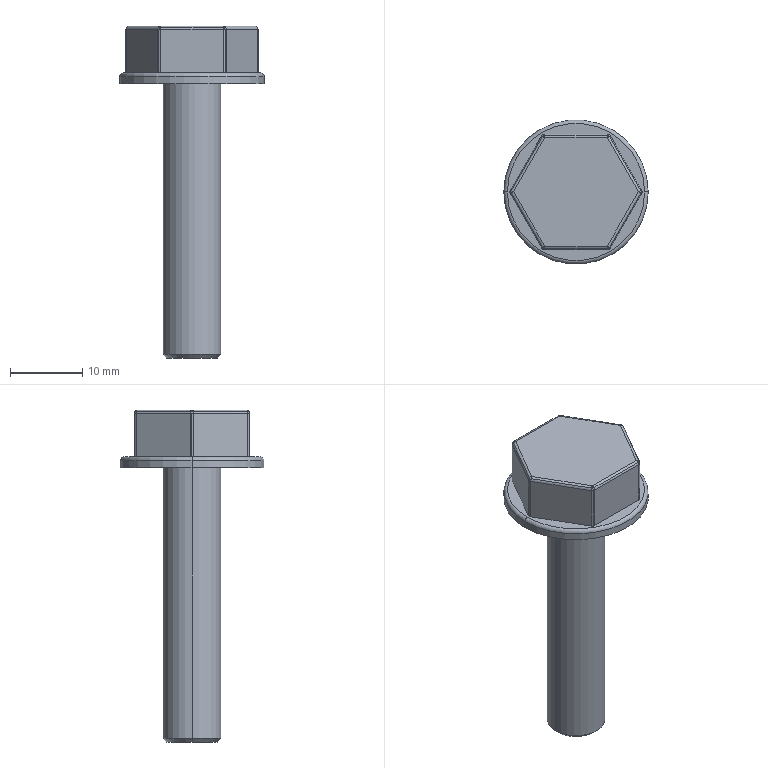Part | SolidWorks | features BaseBody 1 | 1 solid | 54 faces | box 20 x 20 x 46 mm | volume 3813 mm3 | cylinder 28 | sphere 12 | plane 10 | torus 2 | cone 2 | commonest cylinder face diameters 1 x24 8 x2 20 x2
STEP:
#1=CARTESIAN_POINT('',(4.516,-7.964,7.5));
#2=VERTEX_POINT('',#1);
#3=CARTESIAN_POINT('',(4.33,-8.,7.5));
#4=VERTEX_POINT('',#3);
#5=CARTESIAN_POINT('',(4.33,-7.5,7.5));
#6=DIRECTION('',(0.,0.,-1.));
#7=DIRECTION('',(0.866,-0.5,0.));
#8=AXIS2_PLACEMENT_3D('',#5,#6,#7);
#9=CIRCLE('',#8,0.5);
#10=EDGE_CURVE('',#2,#4,#9,.T.);
#11=ORIENTED_EDGE('',*,*,#10,.F.);
#12=CARTESIAN_POINT('',(4.491,-7.593,7.964));
#13=VERTEX_POINT('',#12);
#14=CARTESIAN_POINT('',(4.33,-7.5,7.5));
#15=DIRECTION('',(-0.9014,-0.3603,0.2402));
#16=DIRECTION('',(0.3712,-0.9286,0.));
#17=AXIS2_PLACEMENT_3D('',#14,#15,#16);
#18=CIRCLE('',#17,0.5);
#19=EDGE_CURVE('',#2,#13,#18,.T.);
#20=ORIENTED_EDGE('',*,*,#19,.T.);
#21=CARTESIAN_POINT('',(4.33,-7.5,8.));
#22=VERTEX_POINT('',#21);
#23=CARTESIAN_POINT('',(4.33,-7.5,7.5));
#24=DIRECTION('',(0.5,0.866,0.));
#25=DIRECTION('',(0.,0.,1.));
#26=AXIS2_PLACEMENT_3D('',#23,#24,#25);
#27=CIRCLE('',#26,0.5);
#28=EDGE_CURVE('',#22,#13,#27,.T.);
#29=ORIENTED_EDGE('',*,*,#28,.F.);
#30=CARTESIAN_POINT('',(4.33,-7.854,7.854));
#31=VERTEX_POINT('',#30);
#32=CARTESIAN_POINT('',(4.33,-7.5,7.5));
#33=DIRECTION('',(-1.,0.,0.));
#34=DIRECTION('',(0.,-1.,0.));
#35=AXIS2_PLACEMENT_3D('',#32,#33,#34);
#36=CIRCLE('',#35,0.5);
#37=EDGE_CURVE('',#31,#22,#36,.T.);
#38=ORIENTED_EDGE('',*,*,#37,.F.);
#39=CARTESIAN_POINT('',(4.33,-7.5,7.5));
#40=DIRECTION('',(-1.,0.,0.));
#41=DIRECTION('',(0.,-1.,0.));
#42=AXIS2_PLACEMENT_3D('',#39,#40,#41);
#43=CIRCLE('',#42,0.5);
#44=EDGE_CURVE('',#4,#31,#43,.T.);
#45=ORIENTED_EDGE('',*,*,#44,.F.);
#46=EDGE_LOOP('',(#11,#20,#29,#38,#45));
#47=FACE_OUTER_BOUND('',#46,.T.);
#48=CARTESIAN_POINT('',(4.33,-7.5,7.5));
#49=DIRECTION('',(0.9014,0.3603,-0.2402));
#50=DIRECTION('',(0.433,-0.75,0.5));
#51=AXIS2_PLACEMENT_3D('',#48,#49,#50);
#52=SPHERICAL_SURFACE('',#51,0.5);
#53=ADVANCED_FACE('',(#47),#52,.T.);
#54=CARTESIAN_POINT('',(4.763,-7.75,7.5));
#55=VERTEX_POINT('',#54);
#56=CARTESIAN_POINT('',(4.58,-7.933,7.5));
#57=VERTEX_POINT('',#56);
#58=CARTESIAN_POINT('',(4.33,-7.5,7.5));
#59=DIRECTION('',(0.,0.,-1.));
#60=DIRECTION('',(0.866,-0.5,0.));
#61=AXIS2_PLACEMENT_3D('',#58,#59,#60);
#62=CIRCLE('',#61,0.5);
#63=EDGE_CURVE('',#55,#57,#62,.T.);
#64=ORIENTED_EDGE('',*,*,#63,.T.);
#65=CARTESIAN_POINT('',(4.58,-7.933,1.5));
#66=VERTEX_POINT('',#65);
#67=CARTESIAN_POINT('',(4.58,-7.933,1.5));
#68=DIRECTION('',(0.,0.,-1.));
#69=VECTOR('',#68,1000.);
#70=LINE('',#67,#69);
#71=EDGE_CURVE('',#57,#66,#70,.T.);
#72=ORIENTED_EDGE('',*,*,#71,.T.);
#73=CARTESIAN_POINT('',(4.763,-7.75,1.5));
#74=VERTEX_POINT('',#73);
#75=CARTESIAN_POINT('',(4.33,-7.5,1.5));
#76=DIRECTION('',(0.,0.,1.));
#77=DIRECTION('',(0.5,-0.866,0.));
#78=AXIS2_PLACEMENT_3D('',#75,#76,#77);
#79=CIRCLE('',#78,0.5);
#80=EDGE_CURVE('',#66,#74,#79,.T.);
#81=ORIENTED_EDGE('',*,*,#80,.T.);
#82=CARTESIAN_POINT('',(4.763,-7.75,1.5));
#83=DIRECTION('',(0.,0.,1.));
#84=VECTOR('',#83,1000.);
#85=LINE('',#82,#84);
#86=EDGE_CURVE('',#74,#55,#85,.T.);
#87=ORIENTED_EDGE('',*,*,#86,.T.);
#88=EDGE_LOOP('',(#64,#72,#81,#87));
#89=FACE_OUTER_BOUND('',#88,.T.);
#90=CARTESIAN_POINT('',(4.33,-7.5,1.5));
#91=DIRECTION('',(0.,0.,-1.));
#92=DIRECTION('',(0.5,-0.866,0.));
#93=AXIS2_PLACEMENT_3D('',#90,#91,#92);
#94=CYLINDRICAL_SURFACE('',#93,0.5);
#95=ADVANCED_FACE('',(#89),#94,.T.);
#96=CARTESIAN_POINT('',(-4.516,-7.964,7.5));
#97=VERTEX_POINT('',#96);
#98=CARTESIAN_POINT('',(-4.58,-7.933,7.5));
#99=VERTEX_POINT('',#98);
#100=CARTESIAN_POINT('',(-4.33,-7.5,7.5));
#101=DIRECTION('',(0.,0.,-1.));
#102=DIRECTION('',(0.,-1.,0.));
#103=AXIS2_PLACEMENT_3D('',#100,#101,#102);
#104=CIRCLE('',#103,0.5);
#105=EDGE_CURVE('',#97,#99,#104,.T.);
#106=ORIENTED_EDGE('',*,*,#105,.F.);
#107=CARTESIAN_POINT('',(-4.491,-7.593,7.964));
#108=VERTEX_POINT('',#107);
#109=CARTESIAN_POINT('',(-4.33,-7.5,7.5));
#110=DIRECTION('',(-0.9014,0.3603,-0.2402));
#111=DIRECTION('',(-0.3712,-0.9286,0.));
#112=AXIS2_PLACEMENT_3D('',#109,#110,#111);
#113=CIRCLE('',#112,0.5);
#114=EDGE_CURVE('',#97,#108,#113,.T.);
#115=ORIENTED_EDGE('',*,*,#114,.T.);
#116=CARTESIAN_POINT('',(-4.636,-7.677,7.854));
#117=VERTEX_POINT('',#116);
#118=CARTESIAN_POINT('',(-4.33,-7.5,7.5));
#119=DIRECTION('',(-0.5,0.866,0.));
#120=DIRECTION('',(-0.866,-0.5,0.));
#121=AXIS2_PLACEMENT_3D('',#118,#119,#120);
#122=CIRCLE('',#121,0.5);
#123=EDGE_CURVE('',#117,#108,#122,.T.);
#124=ORIENTED_EDGE('',*,*,#123,.F.);
#125=CARTESIAN_POINT('',(-4.763,-7.75,7.5));
#126=VERTEX_POINT('',#125);
#127=CARTESIAN_POINT('',(-4.33,-7.5,7.5));
#128=DIRECTION('',(-0.5,0.866,0.));
#129=DIRECTION('',(-0.866,-0.5,0.));
#130=AXIS2_PLACEMENT_3D('',#127,#128,#129);
#131=CIRCLE('',#130,0.5);
#132=EDGE_CURVE('',#126,#117,#131,.T.);
#133=ORIENTED_EDGE('',*,*,#132,.F.);
#134=CARTESIAN_POINT('',(-4.33,-7.5,7.5));
#135=DIRECTION('',(0.,0.,-1.));
#136=DIRECTION('',(0.,-1.,0.));
#137=AXIS2_PLACEMENT_3D('',#134,#135,#136);
#138=CIRCLE('',#137,0.5);
#139=EDGE_CURVE('',#99,#126,#138,.T.);
#140=ORIENTED_EDGE('',*,*,#139,.F.);
#141=EDGE_LOOP('',(#106,#115,#124,#133,#140));
#142=FACE_OUTER_BOUND('',#141,.T.);
#143=CARTESIAN_POINT('',(-4.33,-7.5,7.5));
#144=DIRECTION('',(0.9014,-0.3603,0.2402));
#145=DIRECTION('',(-0.433,-0.75,0.5));
#146=AXIS2_PLACEMENT_3D('',#143,#144,#145);
#147=SPHERICAL_SURFACE('',#146,0.5);
#148=ADVANCED_FACE('',(#142),#147,.T.);
#149=CARTESIAN_POINT('',(-4.33,-8.,7.5));
#150=VERTEX_POINT('',#149);
#151=CARTESIAN_POINT('',(-4.33,-7.5,7.5));
#152=DIRECTION('',(0.,0.,-1.));
#153=DIRECTION('',(0.,-1.,0.));
#154=AXIS2_PLACEMENT_3D('',#151,#152,#153);
#155=CIRCLE('',#154,0.5);
#156=EDGE_CURVE('',#150,#97,#155,.T.);
#157=ORIENTED_EDGE('',*,*,#156,.T.);
#158=ORIENTED_EDGE('',*,*,#105,.T.);
#159=CARTESIAN_POINT('',(-4.58,-7.933,1.5));
#160=VERTEX_POINT('',#159);
#161=CARTESIAN_POINT('',(-4.58,-7.933,1.5));
#162=DIRECTION('',(0.,0.,-1.));
#163=VECTOR('',#162,1000.);
#164=LINE('',#161,#163);
#165=EDGE_CURVE('',#99,#160,#164,.T.);
#166=ORIENTED_EDGE('',*,*,#165,.T.);
#167=CARTESIAN_POINT('',(-4.33,-8.,1.5));
#168=VERTEX_POINT('',#167);
#169=CARTESIAN_POINT('',(-4.33,-7.5,1.5));
#170=DIRECTION('',(0.,0.,1.));
#171=DIRECTION('',(-0.5,-0.866,0.));
#172=AXIS2_PLACEMENT_3D('',#169,#170,#171);
#173=CIRCLE('',#172,0.5);
#174=EDGE_CURVE('',#160,#168,#173,.T.);
#175=ORIENTED_EDGE('',*,*,#174,.T.);
#176=CARTESIAN_POINT('',(-4.33,-8.,1.5));
#177=DIRECTION('',(0.,0.,1.));
#178=VECTOR('',#177,1000.);
#179=LINE('',#176,#178);
#180=EDGE_CURVE('',#168,#150,#179,.T.);
#181=ORIENTED_EDGE('',*,*,#180,.T.);
#182=EDGE_LOOP('',(#157,#158,#166,#175,#181));
#183=FACE_OUTER_BOUND('',#182,.T.);
#184=CARTESIAN_POINT('',(-4.33,-7.5,1.5));
#185=DIRECTION('',(0.,0.,-1.));
#186=DIRECTION('',(-0.5,-0.866,0.));
#187=AXIS2_PLACEMENT_3D('',#184,#185,#186);
#188=CYLINDRICAL_SURFACE('',#187,0.5);
#189=ADVANCED_FACE('',(#183),#188,.T.);
#190=ORIENTED_EDGE('',*,*,#44,.T.);
#191=CARTESIAN_POINT('',(-4.33,-7.854,7.854));
#192=VERTEX_POINT('',#191);
#193=CARTESIAN_POINT('',(-2.309,-7.854,7.854));
#194=DIRECTION('',(-1.,0.,0.));
#195=VECTOR('',#194,1000.);
#196=LINE('',#193,#195);
#197=EDGE_CURVE('',#31,#192,#196,.T.);
#198=ORIENTED_EDGE('',*,*,#197,.T.);
#199=CARTESIAN_POINT('',(-4.33,-7.5,7.5));
#200=DIRECTION('',(1.,0.,0.));
#201=DIRECTION('',(0.,0.,1.));
#202=AXIS2_PLACEMENT_3D('',#199,#200,#201);
#203=CIRCLE('',#202,0.5);
#204=EDGE_CURVE('',#192,#150,#203,.T.);
#205=ORIENTED_EDGE('',*,*,#204,.T.);
#206=CARTESIAN_POINT('',(-2.309,-8.,7.5));
#207=DIRECTION('',(1.,0.,0.));
#208=VECTOR('',#207,1000.);
#209=LINE('',#206,#208);
#210=EDGE_CURVE('',#150,#4,#209,.T.);
#211=ORIENTED_EDGE('',*,*,#210,.T.);
#212=EDGE_LOOP('',(#190,#198,#205,#211));
#213=FACE_OUTER_BOUND('',#212,.T.);
#214=CARTESIAN_POINT('',(-2.309,-7.5,7.5));
#215=DIRECTION('',(-1.,0.,0.));
#216=DIRECTION('',(0.,-0.7071,0.7071));
#217=AXIS2_PLACEMENT_3D('',#214,#215,#216);
#218=CYLINDRICAL_SURFACE('',#217,0.5);
#219=ADVANCED_FACE('',(#213),#218,.T.);
#220=CARTESIAN_POINT('',(9.048,0.2236,7.724));
#221=VERTEX_POINT('',#220);
#222=CARTESIAN_POINT('',(9.093,0.25,7.5));
#223=VERTEX_POINT('',#222);
#224=CARTESIAN_POINT('',(8.66,0.,7.5));
#225=DIRECTION('',(-0.5,0.866,0.));
#226=DIRECTION('',(0.,0.,1.));
#227=AXIS2_PLACEMENT_3D('',#224,#225,#226);
#228=CIRCLE('',#227,0.5);
#229=EDGE_CURVE('',#221,#223,#228,.T.);
#230=ORIENTED_EDGE('',*,*,#229,.F.);
#231=CARTESIAN_POINT('',(9.048,-0.2236,7.724));
#232=VERTEX_POINT('',#231);
#233=CARTESIAN_POINT('',(8.66,0.,7.5));
#234=DIRECTION('',(0.5,0.,-0.866));
#235=DIRECTION('',(-0.866,0.,-0.5));
#236=AXIS2_PLACEMENT_3D('',#233,#234,#235);
#237=CIRCLE('',#236,0.5);
#238=EDGE_CURVE('',#221,#232,#237,.T.);
#239=ORIENTED_EDGE('',*,*,#238,.T.);
#240=CARTESIAN_POINT('',(9.093,-0.25,7.5));
#241=VERTEX_POINT('',#240);
#242=CARTESIAN_POINT('',(8.66,0.,7.5));
#243=DIRECTION('',(-0.5,-0.866,0.));
#244=DIRECTION('',(0.866,-0.5,0.));
#245=AXIS2_PLACEMENT_3D('',#242,#243,#244);
#246=CIRCLE('',#245,0.5);
#247=EDGE_CURVE('',#241,#232,#246,.T.);
#248=ORIENTED_EDGE('',*,*,#247,.F.);
#249=CARTESIAN_POINT('',(9.16,0.,7.5));
#250=VERTEX_POINT('',#249);
#251=CARTESIAN_POINT('',(8.66,0.,7.5));
#252=DIRECTION('',(0.,0.,-1.));
#253=DIRECTION('',(0.866,0.5,0.));
#254=AXIS2_PLACEMENT_3D('',#251,#252,#253);
#255=CIRCLE('',#254,0.5);
#256=EDGE_CURVE('',#250,#241,#255,.T.);
#257=ORIENTED_EDGE('',*,*,#256,.F.);
#258=CARTESIAN_POINT('',(8.66,0.,7.5));
#259=DIRECTION('',(0.,0.,-1.));
#260=DIRECTION('',(0.866,0.5,0.));
#261=AXIS2_PLACEMENT_3D('',#258,#259,#260);
#262=CIRCLE('',#261,0.5);
#263=EDGE_CURVE('',#223,#250,#262,.T.);
#264=ORIENTED_EDGE('',*,*,#263,.F.);
#265=EDGE_LOOP('',(#230,#239,#248,#257,#264));
#266=FACE_OUTER_BOUND('',#265,.T.);
#267=CARTESIAN_POINT('',(8.66,0.,7.5));
#268=DIRECTION('',(-0.5,0.,0.866));
#269=DIRECTION('',(0.866,0.,0.5));
#270=AXIS2_PLACEMENT_3D('',#267,#268,#269);
#271=SPHERICAL_SURFACE('',#270,0.5);
#272=ADVANCED_FACE('',(#266),#271,.T.);
#273=ORIENTED_EDGE('',*,*,#263,.T.);
#274=CARTESIAN_POINT('',(9.16,0.,1.5));
#275=VERTEX_POINT('',#274);
#276=CARTESIAN_POINT('',(9.16,0.,1.5));
#277=DIRECTION('',(0.,0.,-1.));
#278=VECTOR('',#277,1000.);
#279=LINE('',#276,#278);
#280=EDGE_CURVE('',#250,#275,#279,.T.);
#281=ORIENTED_EDGE('',*,*,#280,.T.);
#282=CARTESIAN_POINT('',(9.093,0.25,1.5));
#283=VERTEX_POINT('',#282);
#284=CARTESIAN_POINT('',(8.66,0.,1.5));
#285=DIRECTION('',(0.,0.,1.));
#286=DIRECTION('',(1.,0.,0.));
#287=AXIS2_PLACEMENT_3D('',#284,#285,#286);
#288=CIRCLE('',#287,0.5);
#289=EDGE_CURVE('',#275,#283,#288,.T.);
#290=ORIENTED_EDGE('',*,*,#289,.T.);
#291=CARTESIAN_POINT('',(9.093,0.25,1.5));
#292=DIRECTION('',(0.,0.,1.));
#293=VECTOR('',#292,1000.);
#294=LINE('',#291,#293);
#295=EDGE_CURVE('',#283,#223,#294,.T.);
#296=ORIENTED_EDGE('',*,*,#295,.T.);
#297=EDGE_LOOP('',(#273,#281,#290,#296));
#298=FACE_OUTER_BOUND('',#297,.T.);
#299=CARTESIAN_POINT('',(8.66,0.,1.5));
#300=DIRECTION('',(0.,0.,-1.));
#301=DIRECTION('',(1.,0.,0.));
#302=AXIS2_PLACEMENT_3D('',#299,#300,#301);
#303=CYLINDRICAL_SURFACE('',#302,0.5);
#304=ADVANCED_FACE('',(#298),#303,.T.);
#305=CARTESIAN_POINT('',(-9.048,-0.2236,7.724));
#306=VERTEX_POINT('',#305);
#307=CARTESIAN_POINT('',(-9.093,-0.25,7.5));
#308=VERTEX_POINT('',#307);
#309=CARTESIAN_POINT('',(-8.66,0.,7.5));
#310=DIRECTION('',(0.5,-0.866,0.));
#311=DIRECTION('',(0.,0.,1.));
#312=AXIS2_PLACEMENT_3D('',#309,#310,#311);
#313=CIRCLE('',#312,0.5);
#314=EDGE_CURVE('',#306,#308,#313,.T.);
#315=ORIENTED_EDGE('',*,*,#314,.F.);
#316=CARTESIAN_POINT('',(-9.048,0.2236,7.724));
#317=VERTEX_POINT('',#316);
#318=CARTESIAN_POINT('',(-8.66,0.,7.5));
#319=DIRECTION('',(-0.5,0.,-0.866));
#320=DIRECTION('',(-0.866,0.,0.5));
#321=AXIS2_PLACEMENT_3D('',#318,#319,#320);
#322=CIRCLE('',#321,0.5);
#323=EDGE_CURVE('',#306,#317,#322,.T.);
#324=ORIENTED_EDGE('',*,*,#323,.T.);
#325=CARTESIAN_POINT('',(-9.093,0.25,7.5));
#326=VERTEX_POINT('',#325);
#327=CARTESIAN_POINT('',(-8.66,0.,7.5));
#328=DIRECTION('',(0.5,0.866,0.));
#329=DIRECTION('',(-0.866,0.5,0.));
#330=AXIS2_PLACEMENT_3D('',#327,#328,#329);
#331=CIRCLE('',#330,0.5);
#332=EDGE_CURVE('',#326,#317,#331,.T.);
#333=ORIENTED_EDGE('',*,*,#332,.F.);
#334=CARTESIAN_POINT('',(-9.16,0.,7.5));
#335=VERTEX_POINT('',#334);
#336=CARTESIAN_POINT('',(-8.66,0.,7.5));
#337=DIRECTION('',(0.,0.,-1.));
#338=DIRECTION('',(-0.866,-0.5,0.));
#339=AXIS2_PLACEMENT_3D('',#336,#337,#338);
#340=CIRCLE('',#339,0.5);
#341=EDGE_CURVE('',#335,#326,#340,.T.);
#342=ORIENTED_EDGE('',*,*,#341,.F.);
#343=CARTESIAN_POINT('',(-8.66,0.,7.5));
#344=DIRECTION('',(0.,0.,-1.));
#345=DIRECTION('',(-0.866,-0.5,0.));
#346=AXIS2_PLACEMENT_3D('',#343,#344,#345);
#347=CIRCLE('',#346,0.5);
#348=EDGE_CURVE('',#308,#335,#347,.T.);
#349=ORIENTED_EDGE('',*,*,#348,.F.);
#350=EDGE_LOOP('',(#315,#324,#333,#342,#349));
#351=FACE_OUTER_BOUND('',#350,.T.);
#352=CARTESIAN_POINT('',(-8.66,0.,7.5));
#353=DIRECTION('',(0.5,0.,0.866));
#354=DIRECTION('',(-0.866,0.,0.5));
#355=AXIS2_PLACEMENT_3D('',#352,#353,#354);
#356=SPHERICAL_SURFACE('',#355,0.5);
#357=ADVANCED_FACE('',(#351),#356,.T.);
#358=ORIENTED_EDGE('',*,*,#348,.T.);
#359=CARTESIAN_POINT('',(-9.16,0.,1.5));
#360=VERTEX_POINT('',#359);
#361=CARTESIAN_POINT('',(-9.16,0.,1.5));
#362=DIRECTION('',(0.,0.,-1.));
#363=VECTOR('',#362,1000.);
#364=LINE('',#361,#363);
#365=EDGE_CURVE('',#335,#360,#364,.T.);
#366=ORIENTED_EDGE('',*,*,#365,.T.);
#367=CARTESIAN_POINT('',(-9.093,-0.25,1.5));
#368=VERTEX_POINT('',#367);
#369=CARTESIAN_POINT('',(-8.66,0.,1.5));
#370=DIRECTION('',(0.,0.,1.));
#371=DIRECTION('',(-1.,0.,0.));
#372=AXIS2_PLACEMENT_3D('',#369,#370,#371);
#373=CIRCLE('',#372,0.5);
#374=EDGE_CURVE('',#360,#368,#373,.T.);
#375=ORIENTED_EDGE('',*,*,#374,.T.);
#376=CARTESIAN_POINT('',(-9.093,-0.25,1.5));
#377=DIRECTION('',(0.,0.,1.));
#378=VECTOR('',#377,1000.);
#379=LINE('',#376,#378);
#380=EDGE_CURVE('',#368,#308,#379,.T.);
#381=ORIENTED_EDGE('',*,*,#380,.T.);
#382=EDGE_LOOP('',(#358,#366,#375,#381));
#383=FACE_OUTER_BOUND('',#382,.T.);
#384=CARTESIAN_POINT('',(-8.66,0.,1.5));
#385=DIRECTION('',(0.,0.,-1.));
#386=DIRECTION('',(-1.,0.,0.));
#387=AXIS2_PLACEMENT_3D('',#384,#385,#386);
#388=CYLINDRICAL_SURFACE('',#387,0.5);
#389=ADVANCED_FACE('',(#383),#388,.T.);
#390=ORIENTED_EDGE('',*,*,#132,.T.);
#391=CARTESIAN_POINT('',(-8.966,-0.1768,7.854));
#392=VERTEX_POINT('',#391);
#393=CARTESIAN_POINT('',(-7.956,-1.927,7.854));
#394=DIRECTION('',(-0.5,0.866,0.));
#395=VECTOR('',#394,1000.);
#396=LINE('',#393,#395);
#397=EDGE_CURVE('',#117,#392,#396,.T.);
#398=ORIENTED_EDGE('',*,*,#397,.T.);
#399=CARTESIAN_POINT('',(-8.66,0.,7.5));
#400=DIRECTION('',(0.5,-0.866,0.));
#401=DIRECTION('',(0.,0.,1.));
#402=AXIS2_PLACEMENT_3D('',#399,#400,#401);
#403=CIRCLE('',#402,0.5);
#404=EDGE_CURVE('',#392,#306,#403,.T.);
#405=ORIENTED_EDGE('',*,*,#404,.T.);
#406=ORIENTED_EDGE('',*,*,#314,.T.);
#407=CARTESIAN_POINT('',(-8.083,-2.,7.5));
#408=DIRECTION('',(0.5,-0.866,0.));
#409=VECTOR('',#408,1000.);
#410=LINE('',#407,#409);
#411=EDGE_CURVE('',#308,#126,#410,.T.);
#412=ORIENTED_EDGE('',*,*,#411,.T.);
#413=EDGE_LOOP('',(#390,#398,#405,#406,#412));
#414=FACE_OUTER_BOUND('',#413,.T.);
#415=CARTESIAN_POINT('',(-7.65,-1.75,7.5));
#416=DIRECTION('',(-0.5,0.866,0.));
#417=DIRECTION('',(-0.6124,-0.3536,0.7071));
#418=AXIS2_PLACEMENT_3D('',#415,#416,#417);
#419=CYLINDRICAL_SURFACE('',#418,0.5);
#420=ADVANCED_FACE('',(#414),#419,.T.);
#421=CARTESIAN_POINT('',(4.491,7.593,7.964));
#422=VERTEX_POINT('',#421);
#423=CARTESIAN_POINT('',(4.33,7.5,8.));
#424=VERTEX_POINT('',#423);
#425=CARTESIAN_POINT('',(4.33,7.5,7.5));
#426=DIRECTION('',(0.5,-0.866,0.));
#427=DIRECTION('',(0.866,0.5,0.));
#428=AXIS2_PLACEMENT_3D('',#425,#426,#427);
#429=CIRCLE('',#428,0.5);
#430=EDGE_CURVE('',#422,#424,#429,.T.);
#431=ORIENTED_EDGE('',*,*,#430,.F.);
#432=CARTESIAN_POINT('',(4.516,7.964,7.5));
#433=VERTEX_POINT('',#432);
#434=CARTESIAN_POINT('',(4.33,7.5,7.5));
#435=DIRECTION('',(-0.9014,0.3603,0.2402));
#436=DIRECTION('',(-0.3712,-0.9286,0.));
#437=AXIS2_PLACEMENT_3D('',#434,#435,#436);
#438=CIRCLE('',#437,0.5);
#439=EDGE_CURVE('',#422,#433,#438,.T.);
#440=ORIENTED_EDGE('',*,*,#439,.T.);
#441=CARTESIAN_POINT('',(4.33,8.,7.5));
#442=VERTEX_POINT('',#441);
#443=CARTESIAN_POINT('',(4.33,7.5,7.5));
#444=DIRECTION('',(0.,0.,-1.));
#445=DIRECTION('',(0.,1.,0.));
#446=AXIS2_PLACEMENT_3D('',#443,#444,#445);
#447=CIRCLE('',#446,0.5);
#448=EDGE_CURVE('',#442,#433,#447,.T.);
#449=ORIENTED_EDGE('',*,*,#448,.F.);
#450=CARTESIAN_POINT('',(4.33,7.854,7.854));
#451=VERTEX_POINT('',#450);
#452=CARTESIAN_POINT('',(4.33,7.5,7.5));
#453=DIRECTION('',(-1.,0.,0.));
#454=DIRECTION('',(0.,0.,1.));
#455=AXIS2_PLACEMENT_3D('',#452,#453,#454);
#456=CIRCLE('',#455,0.5);
#457=EDGE_CURVE('',#451,#442,#456,.T.);
#458=ORIENTED_EDGE('',*,*,#457,.F.);
#459=CARTESIAN_POINT('',(4.33,7.5,7.5));
#460=DIRECTION('',(-1.,0.,0.));
#461=DIRECTION('',(0.,0.,1.));
#462=AXIS2_PLACEMENT_3D('',#459,#460,#461);
#463=CIRCLE('',#462,0.5);
#464=EDGE_CURVE('',#424,#451,#463,.T.);
#465=ORIENTED_EDGE('',*,*,#464,.F.);
#466=EDGE_LOOP('',(#431,#440,#449,#458,#465));
#467=FACE_OUTER_BOUND('',#466,.T.);
#468=CARTESIAN_POINT('',(4.33,7.5,7.5));
#469=DIRECTION('',(0.9014,-0.3603,-0.2402));
#470=DIRECTION('',(0.433,0.75,0.5));
#471=AXIS2_PLACEMENT_3D('',#468,#469,#470);
#472=SPHERICAL_SURFACE('',#471,0.5);
#473=ADVANCED_FACE('',(#467),#472,.T.);
#474=ORIENTED_EDGE('',*,*,#448,.T.);
#475=CARTESIAN_POINT('',(4.58,7.933,7.5));
#476=VERTEX_POINT('',#475);
#477=CARTESIAN_POINT('',(4.33,7.5,7.5));
#478=DIRECTION('',(0.,0.,-1.));
#479=DIRECTION('',(0.,1.,0.));
#480=AXIS2_PLACEMENT_3D('',#477,#478,#479);
#481=CIRCLE('',#480,0.5);
#482=EDGE_CURVE('',#433,#476,#481,.T.);
#483=ORIENTED_EDGE('',*,*,#482,.T.);
#484=CARTESIAN_POINT('',(4.58,7.933,1.5));
#485=VERTEX_POINT('',#484);
#486=CARTESIAN_POINT('',(4.58,7.933,1.5));
#487=DIRECTION('',(0.,0.,-1.));
#488=VECTOR('',#487,1000.);
#489=LINE('',#486,#488);
#490=EDGE_CURVE('',#476,#485,#489,.T.);
#491=ORIENTED_EDGE('',*,*,#490,.T.);
#492=CARTESIAN_POINT('',(4.33,8.,1.5));
#493=VERTEX_POINT('',#492);
#494=CARTESIAN_POINT('',(4.33,7.5,1.5));
#495=DIRECTION('',(0.,0.,1.));
#496=DIRECTION('',(0.5,0.866,0.));
#497=AXIS2_PLACEMENT_3D('',#494,#495,#496);
#498=CIRCLE('',#497,0.5);
#499=EDGE_CURVE('',#485,#493,#498,.T.);
#500=ORIENTED_EDGE('',*,*,#499,.T.);
#501=CARTESIAN_POINT('',(4.33,8.,1.5));
#502=DIRECTION('',(0.,0.,1.));
#503=VECTOR('',#502,1000.);
#504=LINE('',#501,#503);
#505=EDGE_CURVE('',#493,#442,#504,.T.);
#506=ORIENTED_EDGE('',*,*,#505,.T.);
#507=EDGE_LOOP('',(#474,#483,#491,#500,#506));
#508=FACE_OUTER_BOUND('',#507,.T.);
#509=CARTESIAN_POINT('',(4.33,7.5,1.5));
#510=DIRECTION('',(0.,0.,-1.));
#511=DIRECTION('',(0.5,0.866,0.));
#512=AXIS2_PLACEMENT_3D('',#509,#510,#511);
#513=CYLINDRICAL_SURFACE('',#512,0.5);
#514=ADVANCED_FACE('',(#508),#513,.T.);
#515=CARTESIAN_POINT('',(-4.491,7.593,7.964));
#516=VERTEX_POINT('',#515);
#517=CARTESIAN_POINT('',(-4.636,7.677,7.854));
#518=VERTEX_POINT('',#517);
#519=CARTESIAN_POINT('',(-4.33,7.5,7.5));
#520=DIRECTION('',(-0.5,-0.866,0.));
#521=DIRECTION('',(0.,0.,1.));
#522=AXIS2_PLACEMENT_3D('',#519,#520,#521);
#523=CIRCLE('',#522,0.5);
#524=EDGE_CURVE('',#516,#518,#523,.T.);
#525=ORIENTED_EDGE('',*,*,#524,.F.);
#526=CARTESIAN_POINT('',(-4.516,7.964,7.5));
#527=VERTEX_POINT('',#526);
#528=CARTESIAN_POINT('',(-4.33,7.5,7.5));
#529=DIRECTION('',(-0.9014,-0.3603,-0.2402));
#530=DIRECTION('',(0.3712,-0.9286,0.));
#531=AXIS2_PLACEMENT_3D('',#528,#529,#530);
#532=CIRCLE('',#531,0.5);
#533=EDGE_CURVE('',#516,#527,#532,.T.);
#534=ORIENTED_EDGE('',*,*,#533,.T.);
#535=CARTESIAN_POINT('',(-4.58,7.933,7.5));
#536=VERTEX_POINT('',#535);
#537=CARTESIAN_POINT('',(-4.33,7.5,7.5));
#538=DIRECTION('',(0.,0.,-1.));
#539=DIRECTION('',(-0.866,0.5,0.));
#540=AXIS2_PLACEMENT_3D('',#537,#538,#539);
#541=CIRCLE('',#540,0.5);
#542=EDGE_CURVE('',#536,#527,#541,.T.);
#543=ORIENTED_EDGE('',*,*,#542,.F.);
#544=CARTESIAN_POINT('',(-4.763,7.75,7.5));
#545=VERTEX_POINT('',#544);
#546=CARTESIAN_POINT('',(-4.33,7.5,7.5));
#547=DIRECTION('',(0.,0.,-1.));
#548=DIRECTION('',(-0.866,0.5,0.));
#549=AXIS2_PLACEMENT_3D('',#546,#547,#548);
#550=CIRCLE('',#549,0.5);
#551=EDGE_CURVE('',#545,#536,#550,.T.);
#552=ORIENTED_EDGE('',*,*,#551,.F.);
#553=CARTESIAN_POINT('',(-4.33,7.5,7.5));
#554=DIRECTION('',(-0.5,-0.866,0.));
#555=DIRECTION('',(0.,0.,1.));
#556=AXIS2_PLACEMENT_3D('',#553,#554,#555);
#557=CIRCLE('',#556,0.5);
#558=EDGE_CURVE('',#518,#545,#557,.T.);
#559=ORIENTED_EDGE('',*,*,#558,.F.);
#560=EDGE_LOOP('',(#525,#534,#543,#552,#559));
#561=FACE_OUTER_BOUND('',#560,.T.);
#562=CARTESIAN_POINT('',(-4.33,7.5,7.5));
#563=DIRECTION('',(0.9014,0.3603,0.2402));
#564=DIRECTION('',(-0.433,0.75,0.5));
#565=AXIS2_PLACEMENT_3D('',#562,#563,#564);
#566=SPHERICAL_SURFACE('',#565,0.5);
#567=ADVANCED_FACE('',(#561),#566,.T.);
#568=ORIENTED_EDGE('',*,*,#551,.T.);
#569=CARTESIAN_POINT('',(-4.58,7.933,1.5));
#570=VERTEX_POINT('',#569);
#571=CARTESIAN_POINT('',(-4.58,7.933,1.5));
#572=DIRECTION('',(0.,0.,-1.));
#573=VECTOR('',#572,1000.);
#574=LINE('',#571,#573);
#575=EDGE_CURVE('',#536,#570,#574,.T.);
#576=ORIENTED_EDGE('',*,*,#575,.T.);
#577=CARTESIAN_POINT('',(-4.763,7.75,1.5));
#578=VERTEX_POINT('',#577);
#579=CARTESIAN_POINT('',(-4.33,7.5,1.5));
#580=DIRECTION('',(0.,0.,1.));
#581=DIRECTION('',(-0.5,0.866,0.));
#582=AXIS2_PLACEMENT_3D('',#579,#580,#581);
#583=CIRCLE('',#582,0.5);
#584=EDGE_CURVE('',#570,#578,#583,.T.);
#585=ORIENTED_EDGE('',*,*,#584,.T.);
#586=CARTESIAN_POINT('',(-4.763,7.75,1.5));
#587=DIRECTION('',(0.,0.,1.));
#588=VECTOR('',#587,1000.);
#589=LINE('',#586,#588);
#590=EDGE_CURVE('',#578,#545,#589,.T.);
#591=ORIENTED_EDGE('',*,*,#590,.T.);
#592=EDGE_LOOP('',(#568,#576,#585,#591));
#593=FACE_OUTER_BOUND('',#592,.T.);
#594=CARTESIAN_POINT('',(-4.33,7.5,1.5));
#595=DIRECTION('',(0.,0.,-1.));
#596=DIRECTION('',(-0.5,0.866,0.));
#597=AXIS2_PLACEMENT_3D('',#594,#595,#596);
#598=CYLINDRICAL_SURFACE('',#597,0.5);
#599=ADVANCED_FACE('',(#593),#598,.T.);
#600=ORIENTED_EDGE('',*,*,#332,.T.);
#601=CARTESIAN_POINT('',(-8.966,0.1768,7.854));
#602=VERTEX_POINT('',#601);
#603=CARTESIAN_POINT('',(-8.66,0.,7.5));
#604=DIRECTION('',(0.5,0.866,0.));
#605=DIRECTION('',(-0.866,0.5,0.));
#606=AXIS2_PLACEMENT_3D('',#603,#604,#605);
#607=CIRCLE('',#606,0.5);
#608=EDGE_CURVE('',#317,#602,#607,.T.);
#609=ORIENTED_EDGE('',*,*,#608,.T.);
#610=CARTESIAN_POINT('',(-5.647,5.927,7.854));
#611=DIRECTION('',(0.5,0.866,0.));
#612=VECTOR('',#611,1000.);
#613=LINE('',#610,#612);
#614=EDGE_CURVE('',#602,#518,#613,.T.);
#615=ORIENTED_EDGE('',*,*,#614,.T.);
#616=ORIENTED_EDGE('',*,*,#558,.T.);
#617=CARTESIAN_POINT('',(-5.774,6.,7.5));
#618=DIRECTION('',(-0.5,-0.866,0.));
#619=VECTOR('',#618,1000.);
#620=LINE('',#617,#619);
#621=EDGE_CURVE('',#545,#326,#620,.T.);
#622=ORIENTED_EDGE('',*,*,#621,.T.);
#623=EDGE_LOOP('',(#600,#609,#615,#616,#622));
#624=FACE_OUTER_BOUND('',#623,.T.);
#625=CARTESIAN_POINT('',(-5.34,5.75,7.5));
#626=DIRECTION('',(0.5,0.866,0.));
#627=DIRECTION('',(-0.6124,0.3536,0.7071));
#628=AXIS2_PLACEMENT_3D('',#625,#626,#627);
#629=CYLINDRICAL_SURFACE('',#628,0.5);
#630=ADVANCED_FACE('',(#624),#629,.T.);
#631=CARTESIAN_POINT('',(-4.33,8.,7.5));
#632=VERTEX_POINT('',#631);
#633=CARTESIAN_POINT('',(-4.33,7.854,7.854));
#634=VERTEX_POINT('',#633);
#635=CARTESIAN_POINT('',(-4.33,7.5,7.5));
#636=DIRECTION('',(1.,0.,0.));
#637=DIRECTION('',(0.,1.,0.));
#638=AXIS2_PLACEMENT_3D('',#635,#636,#637);
#639=CIRCLE('',#638,0.5);
#640=EDGE_CURVE('',#632,#634,#639,.T.);
#641=ORIENTED_EDGE('',*,*,#640,.T.);
#642=CARTESIAN_POINT('',(2.309,7.854,7.854));
#643=DIRECTION('',(1.,0.,0.));
#644=VECTOR('',#643,1000.);
#645=LINE('',#642,#644);
#646=EDGE_CURVE('',#634,#451,#645,.T.);
#647=ORIENTED_EDGE('',*,*,#646,.T.);
#648=ORIENTED_EDGE('',*,*,#457,.T.);
#649=CARTESIAN_POINT('',(2.309,8.,7.5));
#650=DIRECTION('',(-1.,0.,0.));
#651=VECTOR('',#650,1000.);
#652=LINE('',#649,#651);
#653=EDGE_CURVE('',#442,#632,#652,.T.);
#654=ORIENTED_EDGE('',*,*,#653,.T.);
#655=EDGE_LOOP('',(#641,#647,#648,#654));
#656=FACE_OUTER_BOUND('',#655,.T.);
#657=CARTESIAN_POINT('',(2.309,7.5,7.5));
#658=DIRECTION('',(1.,0.,0.));
#659=DIRECTION('',(0.,0.7071,0.7071));
#660=AXIS2_PLACEMENT_3D('',#657,#658,#659);
#661=CYLINDRICAL_SURFACE('',#660,0.5);
#662=ADVANCED_FACE('',(#656),#661,.T.);
#663=CARTESIAN_POINT('',(4.763,7.75,7.5));
#664=VERTEX_POINT('',#663);
#665=CARTESIAN_POINT('',(4.636,7.677,7.854));
#666=VERTEX_POINT('',#665);
#667=CARTESIAN_POINT('',(4.33,7.5,7.5));
#668=DIRECTION('',(0.5,-0.866,0.));
#669=DIRECTION('',(0.866,0.5,0.));
#670=AXIS2_PLACEMENT_3D('',#667,#668,#669);
#671=CIRCLE('',#670,0.5);
#672=EDGE_CURVE('',#664,#666,#671,.T.);
#673=ORIENTED_EDGE('',*,*,#672,.T.);
#674=CARTESIAN_POINT('',(8.966,0.1768,7.854));
#675=VERTEX_POINT('',#674);
#676=CARTESIAN_POINT('',(7.956,1.927,7.854));
#677=DIRECTION('',(0.5,-0.866,0.));
#678=VECTOR('',#677,1000.);
#679=LINE('',#676,#678);
#680=EDGE_CURVE('',#666,#675,#679,.T.);
#681=ORIENTED_EDGE('',*,*,#680,.T.);
#682=CARTESIAN_POINT('',(8.66,0.,7.5));
#683=DIRECTION('',(-0.5,0.866,0.));
#684=DIRECTION('',(0.,0.,1.));
#685=AXIS2_PLACEMENT_3D('',#682,#683,#684);
#686=CIRCLE('',#685,0.5);
#687=EDGE_CURVE('',#675,#221,#686,.T.);
#688=ORIENTED_EDGE('',*,*,#687,.T.);
#689=ORIENTED_EDGE('',*,*,#229,.T.);
#690=CARTESIAN_POINT('',(8.083,2.,7.5));
#691=DIRECTION('',(-0.5,0.866,0.));
#692=VECTOR('',#691,1000.);
#693=LINE('',#690,#692);
#694=EDGE_CURVE('',#223,#664,#693,.T.);
#695=ORIENTED_EDGE('',*,*,#694,.T.);
#696=EDGE_LOOP('',(#673,#681,#688,#689,#695));
#697=FACE_OUTER_BOUND('',#696,.T.);
#698=CARTESIAN_POINT('',(7.65,1.75,7.5));
#699=DIRECTION('',(0.5,-0.866,0.));
#700=DIRECTION('',(0.6124,0.3536,0.7071));
#701=AXIS2_PLACEMENT_3D('',#698,#699,#700);
#702=CYLINDRICAL_SURFACE('',#701,0.5);
#703=ADVANCED_FACE('',(#697),#702,.T.);
#704=ORIENTED_EDGE('',*,*,#247,.T.);
#705=CARTESIAN_POINT('',(8.966,-0.1768,7.854));
#706=VERTEX_POINT('',#705);
#707=CARTESIAN_POINT('',(8.66,0.,7.5));
#708=DIRECTION('',(-0.5,-0.866,0.));
#709=DIRECTION('',(0.866,-0.5,0.));
#710=AXIS2_PLACEMENT_3D('',#707,#708,#709);
#711=CIRCLE('',#710,0.5);
#712=EDGE_CURVE('',#232,#706,#711,.T.);
#713=ORIENTED_EDGE('',*,*,#712,.T.);
#714=CARTESIAN_POINT('',(4.636,-7.677,7.854));
#715=VERTEX_POINT('',#714);
#716=CARTESIAN_POINT('',(5.647,-5.927,7.854));
#717=DIRECTION('',(-0.5,-0.866,0.));
#718=VECTOR('',#717,1000.);
#719=LINE('',#716,#718);
#720=EDGE_CURVE('',#706,#715,#719,.T.);
#721=ORIENTED_EDGE('',*,*,#720,.T.);
#722=CARTESIAN_POINT('',(4.33,-7.5,7.5));
#723=DIRECTION('',(0.5,0.866,0.));
#724=DIRECTION('',(0.,0.,1.));
#725=AXIS2_PLACEMENT_3D('',#722,#723,#724);
#726=CIRCLE('',#725,0.5);
#727=EDGE_CURVE('',#715,#55,#726,.T.);
#728=ORIENTED_EDGE('',*,*,#727,.T.);
#729=CARTESIAN_POINT('',(5.774,-6.,7.5));
#730=DIRECTION('',(0.5,0.866,0.));
#731=VECTOR('',#730,1000.);
#732=LINE('',#729,#731);
#733=EDGE_CURVE('',#55,#241,#732,.T.);
#734=ORIENTED_EDGE('',*,*,#733,.T.);
#735=EDGE_LOOP('',(#704,#713,#721,#728,#734));
#736=FACE_OUTER_BOUND('',#735,.T.);
#737=CARTESIAN_POINT('',(5.34,-5.75,7.5));
#738=DIRECTION('',(-0.5,-0.866,0.));
#739=DIRECTION('',(0.6124,-0.3536,0.7071));
#740=AXIS2_PLACEMENT_3D('',#737,#738,#739);
#741=CYLINDRICAL_SURFACE('',#740,0.5);
#742=ADVANCED_FACE('',(#736),#741,.T.);
#743=CARTESIAN_POINT('',(10.,0.,1.));
#744=VERTEX_POINT('',#743);
#745=CARTESIAN_POINT('',(-10.,0.,1.));
#746=VERTEX_POINT('',#745);
#747=CARTESIAN_POINT('',(0.,0.,1.));
#748=DIRECTION('',(0.,0.,1.));
#749=DIRECTION('',(-1.,0.,0.));
#750=AXIS2_PLACEMENT_3D('',#747,#748,#749);
#751=CIRCLE('',#750,10.);
#752=EDGE_CURVE('',#744,#746,#751,.T.);
#753=ORIENTED_EDGE('',*,*,#752,.T.);
#754=CARTESIAN_POINT('',(-9.5,0.,1.5));
#755=VERTEX_POINT('',#754);
#756=CARTESIAN_POINT('',(-9.5,0.,1.));
#757=DIRECTION('',(0.,1.,0.));
#758=DIRECTION('',(-1.,0.,0.));
#759=AXIS2_PLACEMENT_3D('',#756,#757,#758);
#760=CIRCLE('',#759,0.5);
#761=EDGE_CURVE('',#746,#755,#760,.T.);
#762=ORIENTED_EDGE('',*,*,#761,.T.);
#763=CARTESIAN_POINT('',(9.5,0.,1.5));
#764=VERTEX_POINT('',#763);
#765=CARTESIAN_POINT('',(0.,0.,1.5));
#766=DIRECTION('',(0.,0.,-1.));
#767=DIRECTION('',(-1.,0.,0.));
#768=AXIS2_PLACEMENT_3D('',#765,#766,#767);
#769=CIRCLE('',#768,9.5);
#770=EDGE_CURVE('',#755,#764,#769,.T.);
#771=ORIENTED_EDGE('',*,*,#770,.T.);
#772=CARTESIAN_POINT('',(9.5,0.,1.));
#773=DIRECTION('',(0.,-1.,0.));
#774=DIRECTION('',(0.,0.,-1.));
#775=AXIS2_PLACEMENT_3D('',#772,#773,#774);
#776=CIRCLE('',#775,0.5);
#777=EDGE_CURVE('',#744,#764,#776,.T.);
#778=ORIENTED_EDGE('',*,*,#777,.F.);
#779=EDGE_LOOP('',(#753,#762,#771,#778));
#780=FACE_OUTER_BOUND('',#779,.T.);
#781=CARTESIAN_POINT('',(0.,0.,1.));
#782=DIRECTION('',(0.,0.,1.));
#783=DIRECTION('',(1.,0.,0.));
#784=AXIS2_PLACEMENT_3D('',#781,#782,#783);
#785=TOROIDAL_SURFACE('',#784,9.5,0.5);
#786=ADVANCED_FACE('',(#780),#785,.T.);
#787=ORIENTED_EDGE('',*,*,#752,.F.);
#788=CARTESIAN_POINT('',(10.,0.,0.));
#789=VERTEX_POINT('',#788);
#790=CARTESIAN_POINT('',(10.,0.,0.));
#791=DIRECTION('',(0.,0.,-1.));
#792=VECTOR('',#791,1000.);
#793=LINE('',#790,#792);
#794=EDGE_CURVE('',#744,#789,#793,.T.);
#795=ORIENTED_EDGE('',*,*,#794,.T.);
#796=CARTESIAN_POINT('',(-10.,0.,0.));
#797=VERTEX_POINT('',#796);
#798=CARTESIAN_POINT('',(0.,0.,0.));
#799=DIRECTION('',(0.,0.,-1.));
#800=DIRECTION('',(-1.,0.,0.));
#801=AXIS2_PLACEMENT_3D('',#798,#799,#800);
#802=CIRCLE('',#801,10.);
#803=EDGE_CURVE('',#797,#789,#802,.T.);
#804=ORIENTED_EDGE('',*,*,#803,.F.);
#805=CARTESIAN_POINT('',(-10.,0.,0.));
#806=DIRECTION('',(0.,0.,-1.));
#807=VECTOR('',#806,1000.);
#808=LINE('',#805,#807);
#809=EDGE_CURVE('',#746,#797,#808,.T.);
#810=ORIENTED_EDGE('',*,*,#809,.F.);
#811=EDGE_LOOP('',(#787,#795,#804,#810));
#812=FACE_OUTER_BOUND('',#811,.T.);
#813=CARTESIAN_POINT('',(0.,0.,0.));
#814=DIRECTION('',(0.,0.,-1.));
#815=DIRECTION('',(-1.,0.,0.));
#816=AXIS2_PLACEMENT_3D('',#813,#814,#815);
#817=CYLINDRICAL_SURFACE('',#816,10.);
#818=ADVANCED_FACE('',(#812),#817,.T.);
#819=CARTESIAN_POINT('',(3.5,0.,-38.));
#820=VERTEX_POINT('',#819);
#821=CARTESIAN_POINT('',(-3.5,0.,-38.));
#822=VERTEX_POINT('',#821);
#823=CARTESIAN_POINT('',(0.,0.,-38.));
#824=DIRECTION('',(0.,0.,1.));
#825=DIRECTION('',(1.,0.,0.));
#826=AXIS2_PLACEMENT_3D('',#823,#824,#825);
#827=CIRCLE('',#826,3.5);
#828=EDGE_CURVE('',#820,#822,#827,.T.);
#829=ORIENTED_EDGE('',*,*,#828,.T.);
#830=CARTESIAN_POINT('',(-4.,0.,-37.5));
#831=VERTEX_POINT('',#830);
#832=CARTESIAN_POINT('',(-3.75,0.,-37.75));
#833=DIRECTION('',(-0.7071,0.,0.7071));
#834=VECTOR('',#833,1000.);
#835=LINE('',#832,#834);
#836=EDGE_CURVE('',#822,#831,#835,.T.);
#837=ORIENTED_EDGE('',*,*,#836,.T.);
#838=CARTESIAN_POINT('',(4.,0.,-37.5));
#839=VERTEX_POINT('',#838);
#840=CARTESIAN_POINT('',(0.,0.,-37.5));
#841=DIRECTION('',(0.,0.,-1.));
#842=DIRECTION('',(1.,0.,0.));
#843=AXIS2_PLACEMENT_3D('',#840,#841,#842);
#844=CIRCLE('',#843,4.);
#845=EDGE_CURVE('',#831,#839,#844,.T.);
#846=ORIENTED_EDGE('',*,*,#845,.T.);
#847=CARTESIAN_POINT('',(3.75,0.,-37.75));
#848=DIRECTION('',(0.7071,0.,0.7071));
#849=VECTOR('',#848,1000.);
#850=LINE('',#847,#849);
#851=EDGE_CURVE('',#820,#839,#850,.T.);
#852=ORIENTED_EDGE('',*,*,#851,.F.);
#853=EDGE_LOOP('',(#829,#837,#846,#852));
#854=FACE_OUTER_BOUND('',#853,.T.);
#855=CARTESIAN_POINT('',(0.,0.,-37.75));
#856=DIRECTION('',(0.,0.,1.));
#857=DIRECTION('',(1.,0.,0.));
#858=AXIS2_PLACEMENT_3D('',#855,#856,#857);
#859=CONICAL_SURFACE('',#858,3.75,0.7854);
#860=ADVANCED_FACE('',(#854),#859,.T.);
#861=ORIENTED_EDGE('',*,*,#845,.F.);
#862=CARTESIAN_POINT('',(-4.,0.,0.));
#863=VERTEX_POINT('',#862);
#864=CARTESIAN_POINT('',(-4.,0.,0.));
#865=DIRECTION('',(0.,0.,1.));
#866=VECTOR('',#865,1000.);
#867=LINE('',#864,#866);
#868=EDGE_CURVE('',#831,#863,#867,.T.);
#869=ORIENTED_EDGE('',*,*,#868,.T.);
#870=CARTESIAN_POINT('',(4.,0.,0.));
#871=VERTEX_POINT('',#870);
#872=CARTESIAN_POINT('',(0.,0.,0.));
#873=DIRECTION('',(0.,0.,1.));
#874=DIRECTION('',(1.,0.,0.));
#875=AXIS2_PLACEMENT_3D('',#872,#873,#874);
#876=CIRCLE('',#875,4.);
#877=EDGE_CURVE('',#871,#863,#876,.T.);
#878=ORIENTED_EDGE('',*,*,#877,.F.);
#879=CARTESIAN_POINT('',(4.,0.,0.));
#880=DIRECTION('',(0.,0.,1.));
#881=VECTOR('',#880,1000.);
#882=LINE('',#879,#881);
#883=EDGE_CURVE('',#839,#871,#882,.T.);
#884=ORIENTED_EDGE('',*,*,#883,.F.);
#885=EDGE_LOOP('',(#861,#869,#878,#884));
#886=FACE_OUTER_BOUND('',#885,.T.);
#887=CARTESIAN_POINT('',(0.,0.,0.));
#888=DIRECTION('',(0.,0.,1.));
#889=DIRECTION('',(1.,0.,0.));
#890=AXIS2_PLACEMENT_3D('',#887,#888,#889);
#891=CYLINDRICAL_SURFACE('',#890,4.);
#892=ADVANCED_FACE('',(#886),#891,.T.);
#893=CARTESIAN_POINT('',(4.33,-8.,1.5));
#894=VERTEX_POINT('',#893);
#895=CARTESIAN_POINT('',(4.33,-8.,1.5));
#896=DIRECTION('',(0.,0.,-1.));
#897=VECTOR('',#896,1000.);
#898=LINE('',#895,#897);
#899=EDGE_CURVE('',#4,#894,#898,.T.);
#900=ORIENTED_EDGE('',*,*,#899,.F.);
#901=ORIENTED_EDGE('',*,*,#210,.F.);
#902=ORIENTED_EDGE('',*,*,#180,.F.);
#903=CARTESIAN_POINT('',(-2.309,-8.,1.5));
#904=DIRECTION('',(-1.,0.,0.));
#905=VECTOR('',#904,1000.);
#906=LINE('',#903,#905);
#907=EDGE_CURVE('',#894,#168,#906,.T.);
#908=ORIENTED_EDGE('',*,*,#907,.F.);
#909=EDGE_LOOP('',(#900,#901,#902,#908));
#910=FACE_OUTER_BOUND('',#909,.T.);
#911=CARTESIAN_POINT('',(-4.619,-8.,1.5));
#912=DIRECTION('',(0.,-1.,0.));
#913=DIRECTION('',(-1.,0.,0.));
#914=AXIS2_PLACEMENT_3D('',#911,#912,#913);
#915=PLANE('',#914);
#916=ADVANCED_FACE('',(#910),#915,.T.);
#917=CARTESIAN_POINT('',(-4.763,-7.75,1.5));
#918=VERTEX_POINT('',#917);
#919=CARTESIAN_POINT('',(-4.763,-7.75,1.5));
#920=DIRECTION('',(0.,0.,-1.));
#921=VECTOR('',#920,1000.);
#922=LINE('',#919,#921);
#923=EDGE_CURVE('',#126,#918,#922,.T.);
#924=ORIENTED_EDGE('',*,*,#923,.F.);
#925=ORIENTED_EDGE('',*,*,#411,.F.);
#926=ORIENTED_EDGE('',*,*,#380,.F.);
#927=CARTESIAN_POINT('',(-8.083,-2.,1.5));
#928=DIRECTION('',(-0.5,0.866,0.));
#929=VECTOR('',#928,1000.);
#930=LINE('',#927,#929);
#931=EDGE_CURVE('',#918,#368,#930,.T.);
#932=ORIENTED_EDGE('',*,*,#931,.F.);
#933=EDGE_LOOP('',(#924,#925,#926,#932));
#934=FACE_OUTER_BOUND('',#933,.T.);
#935=CARTESIAN_POINT('',(-9.238,0.,1.5));
#936=DIRECTION('',(-0.866,-0.5,0.));
#937=DIRECTION('',(-0.5,0.866,0.));
#938=AXIS2_PLACEMENT_3D('',#935,#936,#937);
#939=PLANE('',#938);
#940=ADVANCED_FACE('',(#934),#939,.T.);
#941=CARTESIAN_POINT('',(-9.093,0.25,1.5));
#942=VERTEX_POINT('',#941);
#943=CARTESIAN_POINT('',(-9.093,0.25,1.5));
#944=DIRECTION('',(0.,0.,-1.));
#945=VECTOR('',#944,1000.);
#946=LINE('',#943,#945);
#947=EDGE_CURVE('',#326,#942,#946,.T.);
#948=ORIENTED_EDGE('',*,*,#947,.F.);
#949=ORIENTED_EDGE('',*,*,#621,.F.);
#950=ORIENTED_EDGE('',*,*,#590,.F.);
#951=CARTESIAN_POINT('',(-5.774,6.,1.5));
#952=DIRECTION('',(0.5,0.866,0.));
#953=VECTOR('',#952,1000.);
#954=LINE('',#951,#953);
#955=EDGE_CURVE('',#942,#578,#954,.T.);
#956=ORIENTED_EDGE('',*,*,#955,.F.);
#957=EDGE_LOOP('',(#948,#949,#950,#956));
#958=FACE_OUTER_BOUND('',#957,.T.);
#959=CARTESIAN_POINT('',(-4.619,8.,1.5));
#960=DIRECTION('',(-0.866,0.5,0.));
#961=DIRECTION('',(0.,0.,1.));
#962=AXIS2_PLACEMENT_3D('',#959,#960,#961);
#963=PLANE('',#962);
#964=ADVANCED_FACE('',(#958),#963,.T.);
#965=CARTESIAN_POINT('',(-4.33,-7.5,8.));
#966=VERTEX_POINT('',#965);
#967=CARTESIAN_POINT('',(-2.309,-7.5,8.));
#968=DIRECTION('',(-1.,0.,0.));
#969=VECTOR('',#968,1000.);
#970=LINE('',#967,#969);
#971=EDGE_CURVE('',#22,#966,#970,.T.);
#972=ORIENTED_EDGE('',*,*,#971,.F.);
#973=CARTESIAN_POINT('',(8.66,0.,8.));
#974=VERTEX_POINT('',#973);
#975=CARTESIAN_POINT('',(5.34,-5.75,8.));
#976=DIRECTION('',(-0.5,-0.866,0.));
#977=VECTOR('',#976,1000.);
#978=LINE('',#975,#977);
#979=EDGE_CURVE('',#974,#22,#978,.T.);
#980=ORIENTED_EDGE('',*,*,#979,.F.);
#981=CARTESIAN_POINT('',(7.65,1.75,8.));
#982=DIRECTION('',(0.5,-0.866,0.));
#983=VECTOR('',#982,1000.);
#984=LINE('',#981,#983);
#985=EDGE_CURVE('',#424,#974,#984,.T.);
#986=ORIENTED_EDGE('',*,*,#985,.F.);
#987=CARTESIAN_POINT('',(-4.33,7.5,8.));
#988=VERTEX_POINT('',#987);
#989=CARTESIAN_POINT('',(2.309,7.5,8.));
#990=DIRECTION('',(1.,0.,0.));
#991=VECTOR('',#990,1000.);
#992=LINE('',#989,#991);
#993=EDGE_CURVE('',#988,#424,#992,.T.);
#994=ORIENTED_EDGE('',*,*,#993,.F.);
#995=CARTESIAN_POINT('',(-8.66,0.,8.));
#996=VERTEX_POINT('',#995);
#997=CARTESIAN_POINT('',(-5.34,5.75,8.));
#998=DIRECTION('',(0.5,0.866,0.));
#999=VECTOR('',#998,1000.);
#1000=LINE('',#997,#999);
#1001=EDGE_CURVE('',#996,#988,#1000,.T.);
#1002=ORIENTED_EDGE('',*,*,#1001,.F.);
#1003=CARTESIAN_POINT('',(-7.65,-1.75,8.));
#1004=DIRECTION('',(-0.5,0.866,0.));
#1005=VECTOR('',#1004,1000.);
#1006=LINE('',#1003,#1005);
#1007=EDGE_CURVE('',#966,#996,#1006,.T.);
#1008=ORIENTED_EDGE('',*,*,#1007,.F.);
#1009=EDGE_LOOP('',(#972,#980,#986,#994,#1002,#1008));
#1010=FACE_OUTER_BOUND('',#1009,.T.);
#1011=CARTESIAN_POINT('',(0.,0.,8.));
#1012=DIRECTION('',(0.,0.,1.));
#1013=DIRECTION('',(1.,0.,0.));
#1014=AXIS2_PLACEMENT_3D('',#1011,#1012,#1013);
#1015=PLANE('',#1014);
#1016=ADVANCED_FACE('',(#1010),#1015,.T.);
#1017=ORIENTED_EDGE('',*,*,#931,.T.);
#1018=ORIENTED_EDGE('',*,*,#374,.F.);
#1019=CARTESIAN_POINT('',(-8.66,0.,1.5));
#1020=DIRECTION('',(0.,0.,1.));
#1021=DIRECTION('',(-1.,0.,0.));
#1022=AXIS2_PLACEMENT_3D('',#1019,#1020,#1021);
#1023=CIRCLE('',#1022,0.5);
#1024=EDGE_CURVE('',#942,#360,#1023,.T.);
#1025=ORIENTED_EDGE('',*,*,#1024,.F.);
#1026=ORIENTED_EDGE('',*,*,#955,.T.);
#1027=ORIENTED_EDGE('',*,*,#584,.F.);
#1028=CARTESIAN_POINT('',(-4.33,8.,1.5));
#1029=VERTEX_POINT('',#1028);
#1030=CARTESIAN_POINT('',(-4.33,7.5,1.5));
#1031=DIRECTION('',(0.,0.,1.));
#1032=DIRECTION('',(-0.5,0.866,0.));
#1033=AXIS2_PLACEMENT_3D('',#1030,#1031,#1032);
#1034=CIRCLE('',#1033,0.5);
#1035=EDGE_CURVE('',#1029,#570,#1034,.T.);
#1036=ORIENTED_EDGE('',*,*,#1035,.F.);
#1037=CARTESIAN_POINT('',(2.309,8.,1.5));
#1038=DIRECTION('',(1.,0.,0.));
#1039=VECTOR('',#1038,1000.);
#1040=LINE('',#1037,#1039);
#1041=EDGE_CURVE('',#1029,#493,#1040,.T.);
#1042=ORIENTED_EDGE('',*,*,#1041,.T.);
#1043=ORIENTED_EDGE('',*,*,#499,.F.);
#1044=CARTESIAN_POINT('',(4.763,7.75,1.5));
#1045=VERTEX_POINT('',#1044);
#1046=CARTESIAN_POINT('',(4.33,7.5,1.5));
#1047=DIRECTION('',(0.,0.,1.));
#1048=DIRECTION('',(0.5,0.866,0.));
#1049=AXIS2_PLACEMENT_3D('',#1046,#1047,#1048);
#1050=CIRCLE('',#1049,0.5);
#1051=EDGE_CURVE('',#1045,#485,#1050,.T.);
#1052=ORIENTED_EDGE('',*,*,#1051,.F.);
#1053=CARTESIAN_POINT('',(8.083,2.,1.5));
#1054=DIRECTION('',(0.5,-0.866,0.));
#1055=VECTOR('',#1054,1000.);
#1056=LINE('',#1053,#1055);
#1057=EDGE_CURVE('',#1045,#283,#1056,.T.);
#1058=ORIENTED_EDGE('',*,*,#1057,.T.);
#1059=ORIENTED_EDGE('',*,*,#289,.F.);
#1060=CARTESIAN_POINT('',(9.093,-0.25,1.5));
#1061=VERTEX_POINT('',#1060);
#1062=CARTESIAN_POINT('',(8.66,0.,1.5));
#1063=DIRECTION('',(0.,0.,1.));
#1064=DIRECTION('',(1.,0.,0.));
#1065=AXIS2_PLACEMENT_3D('',#1062,#1063,#1064);
#1066=CIRCLE('',#1065,0.5);
#1067=EDGE_CURVE('',#1061,#275,#1066,.T.);
#1068=ORIENTED_EDGE('',*,*,#1067,.F.);
#1069=CARTESIAN_POINT('',(5.774,-6.,1.5));
#1070=DIRECTION('',(-0.5,-0.866,0.));
#1071=VECTOR('',#1070,1000.);
#1072=LINE('',#1069,#1071);
#1073=EDGE_CURVE('',#1061,#74,#1072,.T.);
#1074=ORIENTED_EDGE('',*,*,#1073,.T.);
#1075=ORIENTED_EDGE('',*,*,#80,.F.);
#1076=CARTESIAN_POINT('',(4.33,-7.5,1.5));
#1077=DIRECTION('',(0.,0.,1.));
#1078=DIRECTION('',(0.5,-0.866,0.));
#1079=AXIS2_PLACEMENT_3D('',#1076,#1077,#1078);
#1080=CIRCLE('',#1079,0.5);
#1081=EDGE_CURVE('',#894,#66,#1080,.T.);
#1082=ORIENTED_EDGE('',*,*,#1081,.F.);
#1083=ORIENTED_EDGE('',*,*,#907,.T.);
#1084=ORIENTED_EDGE('',*,*,#174,.F.);
#1085=CARTESIAN_POINT('',(-4.33,-7.5,1.5));
#1086=DIRECTION('',(0.,0.,1.));
#1087=DIRECTION('',(-0.5,-0.866,0.));
#1088=AXIS2_PLACEMENT_3D('',#1085,#1086,#1087);
#1089=CIRCLE('',#1088,0.5);
#1090=EDGE_CURVE('',#918,#160,#1089,.T.);
#1091=ORIENTED_EDGE('',*,*,#1090,.F.);
#1092=EDGE_LOOP('',(#1017,#1018,#1025,#1026,#1027,#1036,#1042,#1043,#1052,#1058,#1059,#1068,#1074,#1075,#1082,#1083,#1084,#1091));
#1093=FACE_BOUND('',#1092,.T.);
#1094=CARTESIAN_POINT('',(0.,0.,1.5));
#1095=DIRECTION('',(0.,0.,-1.));
#1096=DIRECTION('',(-1.,0.,0.));
#1097=AXIS2_PLACEMENT_3D('',#1094,#1095,#1096);
#1098=CIRCLE('',#1097,9.5);
#1099=EDGE_CURVE('',#764,#755,#1098,.T.);
#1100=ORIENTED_EDGE('',*,*,#1099,.F.);
#1101=ORIENTED_EDGE('',*,*,#770,.F.);
#1102=EDGE_LOOP('',(#1100,#1101));
#1103=FACE_OUTER_BOUND('',#1102,.T.);
#1104=CARTESIAN_POINT('',(0.,0.,1.5));
#1105=DIRECTION('',(0.,0.,1.));
#1106=DIRECTION('',(1.,0.,0.));
#1107=AXIS2_PLACEMENT_3D('',#1104,#1105,#1106);
#1108=PLANE('',#1107);
#1109=ADVANCED_FACE('',(#1093,#1103),#1108,.T.);
#1110=ORIENTED_EDGE('',*,*,#828,.F.);
#1111=CARTESIAN_POINT('',(0.,0.,-38.));
#1112=DIRECTION('',(0.,0.,1.));
#1113=DIRECTION('',(1.,0.,0.));
#1114=AXIS2_PLACEMENT_3D('',#1111,#1112,#1113);
#1115=CIRCLE('',#1114,3.5);
#1116=EDGE_CURVE('',#822,#820,#1115,.T.);
#1117=ORIENTED_EDGE('',*,*,#1116,.F.);
#1118=EDGE_LOOP('',(#1110,#1117));
#1119=FACE_OUTER_BOUND('',#1118,.T.);
#1120=CARTESIAN_POINT('',(0.,0.,-38.));
#1121=DIRECTION('',(0.,0.,1.));
#1122=DIRECTION('',(1.,0.,0.));
#1123=AXIS2_PLACEMENT_3D('',#1120,#1121,#1122);
#1124=PLANE('',#1123);
#1125=ADVANCED_FACE('',(#1119),#1124,.F.);
#1126=ORIENTED_EDGE('',*,*,#505,.F.);
#1127=ORIENTED_EDGE('',*,*,#1041,.F.);
#1128=CARTESIAN_POINT('',(-4.33,8.,1.5));
#1129=DIRECTION('',(0.,0.,-1.));
#1130=VECTOR('',#1129,1000.);
#1131=LINE('',#1128,#1130);
#1132=EDGE_CURVE('',#632,#1029,#1131,.T.);
#1133=ORIENTED_EDGE('',*,*,#1132,.F.);
#1134=ORIENTED_EDGE('',*,*,#653,.F.);
#1135=EDGE_LOOP('',(#1126,#1127,#1133,#1134));
#1136=FACE_OUTER_BOUND('',#1135,.T.);
#1137=CARTESIAN_POINT('',(4.619,8.,1.5));
#1138=DIRECTION('',(0.,1.,0.));
#1139=DIRECTION('',(1.,0.,0.));
#1140=AXIS2_PLACEMENT_3D('',#1137,#1138,#1139);
#1141=PLANE('',#1140);
#1142=ADVANCED_FACE('',(#1136),#1141,.T.);
#1143=ORIENTED_EDGE('',*,*,#295,.F.);
#1144=ORIENTED_EDGE('',*,*,#1057,.F.);
#1145=CARTESIAN_POINT('',(4.763,7.75,1.5));
#1146=DIRECTION('',(0.,0.,-1.));
#1147=VECTOR('',#1146,1000.);
#1148=LINE('',#1145,#1147);
#1149=EDGE_CURVE('',#664,#1045,#1148,.T.);
#1150=ORIENTED_EDGE('',*,*,#1149,.F.);
#1151=ORIENTED_EDGE('',*,*,#694,.F.);
#1152=EDGE_LOOP('',(#1143,#1144,#1150,#1151));
#1153=FACE_OUTER_BOUND('',#1152,.T.);
#1154=CARTESIAN_POINT('',(9.238,0.,1.5));
#1155=DIRECTION('',(0.866,0.5,0.));
#1156=DIRECTION('',(0.,0.,-1.));
#1157=AXIS2_PLACEMENT_3D('',#1154,#1155,#1156);
#1158=PLANE('',#1157);
#1159=ADVANCED_FACE('',(#1153),#1158,.T.);
#1160=ORIENTED_EDGE('',*,*,#86,.F.);
#1161=ORIENTED_EDGE('',*,*,#1073,.F.);
#1162=CARTESIAN_POINT('',(9.093,-0.25,1.5));
#1163=DIRECTION('',(0.,0.,-1.));
#1164=VECTOR('',#1163,1000.);
#1165=LINE('',#1162,#1164);
#1166=EDGE_CURVE('',#241,#1061,#1165,.T.);
#1167=ORIENTED_EDGE('',*,*,#1166,.F.);
#1168=ORIENTED_EDGE('',*,*,#733,.F.);
#1169=EDGE_LOOP('',(#1160,#1161,#1167,#1168));
#1170=FACE_OUTER_BOUND('',#1169,.T.);
#1171=CARTESIAN_POINT('',(4.619,-8.,1.5));
#1172=DIRECTION('',(0.866,-0.5,0.));
#1173=DIRECTION('',(0.,0.,-1.));
#1174=AXIS2_PLACEMENT_3D('',#1171,#1172,#1173);
#1175=PLANE('',#1174);
#1176=ADVANCED_FACE('',(#1170),#1175,.T.);
#1177=ORIENTED_EDGE('',*,*,#877,.T.);
#1178=CARTESIAN_POINT('',(0.,0.,0.));
#1179=DIRECTION('',(0.,0.,1.));
#1180=DIRECTION('',(1.,0.,0.));
#1181=AXIS2_PLACEMENT_3D('',#1178,#1179,#1180);
#1182=CIRCLE('',#1181,4.);
#1183=EDGE_CURVE('',#863,#871,#1182,.T.);
#1184=ORIENTED_EDGE('',*,*,#1183,.T.);
#1185=EDGE_LOOP('',(#1177,#1184));
#1186=FACE_BOUND('',#1185,.T.);
#1187=ORIENTED_EDGE('',*,*,#803,.T.);
#1188=CARTESIAN_POINT('',(0.,0.,0.));
#1189=DIRECTION('',(0.,0.,-1.));
#1190=DIRECTION('',(-1.,0.,0.));
#1191=AXIS2_PLACEMENT_3D('',#1188,#1189,#1190);
#1192=CIRCLE('',#1191,10.);
#1193=EDGE_CURVE('',#789,#797,#1192,.T.);
#1194=ORIENTED_EDGE('',*,*,#1193,.T.);
#1195=EDGE_LOOP('',(#1187,#1194));
#1196=FACE_OUTER_BOUND('',#1195,.T.);
#1197=CARTESIAN_POINT('',(0.,0.,0.));
#1198=DIRECTION('',(0.,0.,1.));
#1199=DIRECTION('',(1.,0.,0.));
#1200=AXIS2_PLACEMENT_3D('',#1197,#1198,#1199);
#1201=PLANE('',#1200);
#1202=ADVANCED_FACE('',(#1186,#1196),#1201,.F.);
#1203=ORIENTED_EDGE('',*,*,#868,.F.);
#1204=CARTESIAN_POINT('',(0.,0.,-37.5));
#1205=DIRECTION('',(0.,0.,-1.));
#1206=DIRECTION('',(1.,0.,0.));
#1207=AXIS2_PLACEMENT_3D('',#1204,#1205,#1206);
#1208=CIRCLE('',#1207,4.);
#1209=EDGE_CURVE('',#839,#831,#1208,.T.);
#1210=ORIENTED_EDGE('',*,*,#1209,.F.);
#1211=ORIENTED_EDGE('',*,*,#883,.T.);
#1212=ORIENTED_EDGE('',*,*,#1183,.F.);
#1213=EDGE_LOOP('',(#1203,#1210,#1211,#1212));
#1214=FACE_OUTER_BOUND('',#1213,.T.);
#1215=CARTESIAN_POINT('',(0.,0.,0.));
#1216=DIRECTION('',(0.,0.,1.));
#1217=DIRECTION('',(1.,0.,0.));
#1218=AXIS2_PLACEMENT_3D('',#1215,#1216,#1217);
#1219=CYLINDRICAL_SURFACE('',#1218,4.);
#1220=ADVANCED_FACE('',(#1214),#1219,.T.);
#1221=ORIENTED_EDGE('',*,*,#836,.F.);
#1222=ORIENTED_EDGE('',*,*,#1116,.T.);
#1223=ORIENTED_EDGE('',*,*,#851,.T.);
#1224=ORIENTED_EDGE('',*,*,#1209,.T.);
#1225=EDGE_LOOP('',(#1221,#1222,#1223,#1224));
#1226=FACE_OUTER_BOUND('',#1225,.T.);
#1227=CARTESIAN_POINT('',(0.,0.,-37.75));
#1228=DIRECTION('',(0.,0.,1.));
#1229=DIRECTION('',(1.,0.,0.));
#1230=AXIS2_PLACEMENT_3D('',#1227,#1228,#1229);
#1231=CONICAL_SURFACE('',#1230,3.75,0.7854);
#1232=ADVANCED_FACE('',(#1226),#1231,.T.);
#1233=ORIENTED_EDGE('',*,*,#794,.F.);
#1234=CARTESIAN_POINT('',(0.,0.,1.));
#1235=DIRECTION('',(0.,0.,1.));
#1236=DIRECTION('',(-1.,0.,0.));
#1237=AXIS2_PLACEMENT_3D('',#1234,#1235,#1236);
#1238=CIRCLE('',#1237,10.);
#1239=EDGE_CURVE('',#746,#744,#1238,.T.);
#1240=ORIENTED_EDGE('',*,*,#1239,.F.);
#1241=ORIENTED_EDGE('',*,*,#809,.T.);
#1242=ORIENTED_EDGE('',*,*,#1193,.F.);
#1243=EDGE_LOOP('',(#1233,#1240,#1241,#1242));
#1244=FACE_OUTER_BOUND('',#1243,.T.);
#1245=CARTESIAN_POINT('',(0.,0.,0.));
#1246=DIRECTION('',(0.,0.,-1.));
#1247=DIRECTION('',(-1.,0.,0.));
#1248=AXIS2_PLACEMENT_3D('',#1245,#1246,#1247);
#1249=CYLINDRICAL_SURFACE('',#1248,10.);
#1250=ADVANCED_FACE('',(#1244),#1249,.T.);
#1251=ORIENTED_EDGE('',*,*,#761,.F.);
#1252=ORIENTED_EDGE('',*,*,#1239,.T.);
#1253=ORIENTED_EDGE('',*,*,#777,.T.);
#1254=ORIENTED_EDGE('',*,*,#1099,.T.);
#1255=EDGE_LOOP('',(#1251,#1252,#1253,#1254));
#1256=FACE_OUTER_BOUND('',#1255,.T.);
#1257=CARTESIAN_POINT('',(0.,0.,1.));
#1258=DIRECTION('',(0.,0.,1.));
#1259=DIRECTION('',(1.,0.,0.));
#1260=AXIS2_PLACEMENT_3D('',#1257,#1258,#1259);
#1261=TOROIDAL_SURFACE('',#1260,9.5,0.5);
#1262=ADVANCED_FACE('',(#1256),#1261,.T.);
#1263=ORIENTED_EDGE('',*,*,#720,.F.);
#1264=CARTESIAN_POINT('',(8.66,0.,7.5));
#1265=DIRECTION('',(-0.5,-0.866,0.));
#1266=DIRECTION('',(0.866,-0.5,0.));
#1267=AXIS2_PLACEMENT_3D('',#1264,#1265,#1266);
#1268=CIRCLE('',#1267,0.5);
#1269=EDGE_CURVE('',#706,#974,#1268,.T.);
#1270=ORIENTED_EDGE('',*,*,#1269,.T.);
#1271=ORIENTED_EDGE('',*,*,#979,.T.);
#1272=ORIENTED_EDGE('',*,*,#28,.T.);
#1273=CARTESIAN_POINT('',(4.33,-7.5,7.5));
#1274=DIRECTION('',(0.5,0.866,0.));
#1275=DIRECTION('',(0.,0.,1.));
#1276=AXIS2_PLACEMENT_3D('',#1273,#1274,#1275);
#1277=CIRCLE('',#1276,0.5);
#1278=EDGE_CURVE('',#13,#715,#1277,.T.);
#1279=ORIENTED_EDGE('',*,*,#1278,.T.);
#1280=EDGE_LOOP('',(#1263,#1270,#1271,#1272,#1279));
#1281=FACE_OUTER_BOUND('',#1280,.T.);
#1282=CARTESIAN_POINT('',(5.34,-5.75,7.5));
#1283=DIRECTION('',(-0.5,-0.866,0.));
#1284=DIRECTION('',(0.6124,-0.3536,0.7071));
#1285=AXIS2_PLACEMENT_3D('',#1282,#1283,#1284);
#1286=CYLINDRICAL_SURFACE('',#1285,0.5);
#1287=ADVANCED_FACE('',(#1281),#1286,.T.);
#1288=ORIENTED_EDGE('',*,*,#680,.F.);
#1289=CARTESIAN_POINT('',(4.33,7.5,7.5));
#1290=DIRECTION('',(0.5,-0.866,0.));
#1291=DIRECTION('',(0.866,0.5,0.));
#1292=AXIS2_PLACEMENT_3D('',#1289,#1290,#1291);
#1293=CIRCLE('',#1292,0.5);
#1294=EDGE_CURVE('',#666,#422,#1293,.T.);
#1295=ORIENTED_EDGE('',*,*,#1294,.T.);
#1296=ORIENTED_EDGE('',*,*,#430,.T.);
#1297=ORIENTED_EDGE('',*,*,#985,.T.);
#1298=CARTESIAN_POINT('',(8.66,0.,7.5));
#1299=DIRECTION('',(-0.5,0.866,0.));
#1300=DIRECTION('',(0.,0.,1.));
#1301=AXIS2_PLACEMENT_3D('',#1298,#1299,#1300);
#1302=CIRCLE('',#1301,0.5);
#1303=EDGE_CURVE('',#974,#675,#1302,.T.);
#1304=ORIENTED_EDGE('',*,*,#1303,.T.);
#1305=EDGE_LOOP('',(#1288,#1295,#1296,#1297,#1304));
#1306=FACE_OUTER_BOUND('',#1305,.T.);
#1307=CARTESIAN_POINT('',(7.65,1.75,7.5));
#1308=DIRECTION('',(0.5,-0.866,0.));
#1309=DIRECTION('',(0.6124,0.3536,0.7071));
#1310=AXIS2_PLACEMENT_3D('',#1307,#1308,#1309);
#1311=CYLINDRICAL_SURFACE('',#1310,0.5);
#1312=ADVANCED_FACE('',(#1306),#1311,.T.);
#1313=ORIENTED_EDGE('',*,*,#646,.F.);
#1314=CARTESIAN_POINT('',(-4.33,7.5,7.5));
#1315=DIRECTION('',(1.,0.,0.));
#1316=DIRECTION('',(0.,1.,0.));
#1317=AXIS2_PLACEMENT_3D('',#1314,#1315,#1316);
#1318=CIRCLE('',#1317,0.5);
#1319=EDGE_CURVE('',#634,#988,#1318,.T.);
#1320=ORIENTED_EDGE('',*,*,#1319,.T.);
#1321=ORIENTED_EDGE('',*,*,#993,.T.);
#1322=ORIENTED_EDGE('',*,*,#464,.T.);
#1323=EDGE_LOOP('',(#1313,#1320,#1321,#1322));
#1324=FACE_OUTER_BOUND('',#1323,.T.);
#1325=CARTESIAN_POINT('',(2.309,7.5,7.5));
#1326=DIRECTION('',(1.,0.,0.));
#1327=DIRECTION('',(0.,0.7071,0.7071));
#1328=AXIS2_PLACEMENT_3D('',#1325,#1326,#1327);
#1329=CYLINDRICAL_SURFACE('',#1328,0.5);
#1330=ADVANCED_FACE('',(#1324),#1329,.T.);
#1331=ORIENTED_EDGE('',*,*,#614,.F.);
#1332=CARTESIAN_POINT('',(-8.66,0.,7.5));
#1333=DIRECTION('',(0.5,0.866,0.));
#1334=DIRECTION('',(-0.866,0.5,0.));
#1335=AXIS2_PLACEMENT_3D('',#1332,#1333,#1334);
#1336=CIRCLE('',#1335,0.5);
#1337=EDGE_CURVE('',#602,#996,#1336,.T.);
#1338=ORIENTED_EDGE('',*,*,#1337,.T.);
#1339=ORIENTED_EDGE('',*,*,#1001,.T.);
#1340=CARTESIAN_POINT('',(-4.33,7.5,7.5));
#1341=DIRECTION('',(-0.5,-0.866,0.));
#1342=DIRECTION('',(0.,0.,1.));
#1343=AXIS2_PLACEMENT_3D('',#1340,#1341,#1342);
#1344=CIRCLE('',#1343,0.5);
#1345=EDGE_CURVE('',#988,#516,#1344,.T.);
#1346=ORIENTED_EDGE('',*,*,#1345,.T.);
#1347=ORIENTED_EDGE('',*,*,#524,.T.);
#1348=EDGE_LOOP('',(#1331,#1338,#1339,#1346,#1347));
#1349=FACE_OUTER_BOUND('',#1348,.T.);
#1350=CARTESIAN_POINT('',(-5.34,5.75,7.5));
#1351=DIRECTION('',(0.5,0.866,0.));
#1352=DIRECTION('',(-0.6124,0.3536,0.7071));
#1353=AXIS2_PLACEMENT_3D('',#1350,#1351,#1352);
#1354=CYLINDRICAL_SURFACE('',#1353,0.5);
#1355=ADVANCED_FACE('',(#1349),#1354,.T.);
#1356=ORIENTED_EDGE('',*,*,#575,.F.);
#1357=ORIENTED_EDGE('',*,*,#542,.T.);
#1358=CARTESIAN_POINT('',(-4.33,7.5,7.5));
#1359=DIRECTION('',(0.,0.,-1.));
#1360=DIRECTION('',(-0.866,0.5,0.));
#1361=AXIS2_PLACEMENT_3D('',#1358,#1359,#1360);
#1362=CIRCLE('',#1361,0.5);
#1363=EDGE_CURVE('',#527,#632,#1362,.T.);
#1364=ORIENTED_EDGE('',*,*,#1363,.T.);
#1365=ORIENTED_EDGE('',*,*,#1132,.T.);
#1366=ORIENTED_EDGE('',*,*,#1035,.T.);
#1367=EDGE_LOOP('',(#1356,#1357,#1364,#1365,#1366));
#1368=FACE_OUTER_BOUND('',#1367,.T.);
#1369=CARTESIAN_POINT('',(-4.33,7.5,1.5));
#1370=DIRECTION('',(0.,0.,-1.));
#1371=DIRECTION('',(-0.5,0.866,0.));
#1372=AXIS2_PLACEMENT_3D('',#1369,#1370,#1371);
#1373=CYLINDRICAL_SURFACE('',#1372,0.5);
#1374=ADVANCED_FACE('',(#1368),#1373,.T.);
#1375=ORIENTED_EDGE('',*,*,#533,.F.);
#1376=ORIENTED_EDGE('',*,*,#1345,.F.);
#1377=ORIENTED_EDGE('',*,*,#1319,.F.);
#1378=ORIENTED_EDGE('',*,*,#640,.F.);
#1379=ORIENTED_EDGE('',*,*,#1363,.F.);
#1380=EDGE_LOOP('',(#1375,#1376,#1377,#1378,#1379));
#1381=FACE_OUTER_BOUND('',#1380,.T.);
#1382=CARTESIAN_POINT('',(-4.33,7.5,7.5));
#1383=DIRECTION('',(0.9014,0.3603,0.2402));
#1384=DIRECTION('',(-0.433,0.75,0.5));
#1385=AXIS2_PLACEMENT_3D('',#1382,#1383,#1384);
#1386=SPHERICAL_SURFACE('',#1385,0.5);
#1387=ADVANCED_FACE('',(#1381),#1386,.T.);
#1388=ORIENTED_EDGE('',*,*,#490,.F.);
#1389=CARTESIAN_POINT('',(4.33,7.5,7.5));
#1390=DIRECTION('',(0.,0.,-1.));
#1391=DIRECTION('',(0.,1.,0.));
#1392=AXIS2_PLACEMENT_3D('',#1389,#1390,#1391);
#1393=CIRCLE('',#1392,0.5);
#1394=EDGE_CURVE('',#476,#664,#1393,.T.);
#1395=ORIENTED_EDGE('',*,*,#1394,.T.);
#1396=ORIENTED_EDGE('',*,*,#1149,.T.);
#1397=ORIENTED_EDGE('',*,*,#1051,.T.);
#1398=EDGE_LOOP('',(#1388,#1395,#1396,#1397));
#1399=FACE_OUTER_BOUND('',#1398,.T.);
#1400=CARTESIAN_POINT('',(4.33,7.5,1.5));
#1401=DIRECTION('',(0.,0.,-1.));
#1402=DIRECTION('',(0.5,0.866,0.));
#1403=AXIS2_PLACEMENT_3D('',#1400,#1401,#1402);
#1404=CYLINDRICAL_SURFACE('',#1403,0.5);
#1405=ADVANCED_FACE('',(#1399),#1404,.T.);
#1406=ORIENTED_EDGE('',*,*,#439,.F.);
#1407=ORIENTED_EDGE('',*,*,#1294,.F.);
#1408=ORIENTED_EDGE('',*,*,#672,.F.);
#1409=ORIENTED_EDGE('',*,*,#1394,.F.);
#1410=ORIENTED_EDGE('',*,*,#482,.F.);
#1411=EDGE_LOOP('',(#1406,#1407,#1408,#1409,#1410));
#1412=FACE_OUTER_BOUND('',#1411,.T.);
#1413=CARTESIAN_POINT('',(4.33,7.5,7.5));
#1414=DIRECTION('',(0.9014,-0.3603,-0.2402));
#1415=DIRECTION('',(0.433,0.75,0.5));
#1416=AXIS2_PLACEMENT_3D('',#1413,#1414,#1415);
#1417=SPHERICAL_SURFACE('',#1416,0.5);
#1418=ADVANCED_FACE('',(#1412),#1417,.T.);
#1419=ORIENTED_EDGE('',*,*,#397,.F.);
#1420=ORIENTED_EDGE('',*,*,#123,.T.);
#1421=CARTESIAN_POINT('',(-4.33,-7.5,7.5));
#1422=DIRECTION('',(-0.5,0.866,0.));
#1423=DIRECTION('',(-0.866,-0.5,0.));
#1424=AXIS2_PLACEMENT_3D('',#1421,#1422,#1423);
#1425=CIRCLE('',#1424,0.5);
#1426=EDGE_CURVE('',#108,#966,#1425,.T.);
#1427=ORIENTED_EDGE('',*,*,#1426,.T.);
#1428=ORIENTED_EDGE('',*,*,#1007,.T.);
#1429=CARTESIAN_POINT('',(-8.66,0.,7.5));
#1430=DIRECTION('',(0.5,-0.866,0.));
#1431=DIRECTION('',(0.,0.,1.));
#1432=AXIS2_PLACEMENT_3D('',#1429,#1430,#1431);
#1433=CIRCLE('',#1432,0.5);
#1434=EDGE_CURVE('',#996,#392,#1433,.T.);
#1435=ORIENTED_EDGE('',*,*,#1434,.T.);
#1436=EDGE_LOOP('',(#1419,#1420,#1427,#1428,#1435));
#1437=FACE_OUTER_BOUND('',#1436,.T.);
#1438=CARTESIAN_POINT('',(-7.65,-1.75,7.5));
#1439=DIRECTION('',(-0.5,0.866,0.));
#1440=DIRECTION('',(-0.6124,-0.3536,0.7071));
#1441=AXIS2_PLACEMENT_3D('',#1438,#1439,#1440);
#1442=CYLINDRICAL_SURFACE('',#1441,0.5);
#1443=ADVANCED_FACE('',(#1437),#1442,.T.);
#1444=ORIENTED_EDGE('',*,*,#365,.F.);
#1445=ORIENTED_EDGE('',*,*,#341,.T.);
#1446=ORIENTED_EDGE('',*,*,#947,.T.);
#1447=ORIENTED_EDGE('',*,*,#1024,.T.);
#1448=EDGE_LOOP('',(#1444,#1445,#1446,#1447));
#1449=FACE_OUTER_BOUND('',#1448,.T.);
#1450=CARTESIAN_POINT('',(-8.66,0.,1.5));
#1451=DIRECTION('',(0.,0.,-1.));
#1452=DIRECTION('',(-1.,0.,0.));
#1453=AXIS2_PLACEMENT_3D('',#1450,#1451,#1452);
#1454=CYLINDRICAL_SURFACE('',#1453,0.5);
#1455=ADVANCED_FACE('',(#1449),#1454,.T.);
#1456=ORIENTED_EDGE('',*,*,#323,.F.);
#1457=ORIENTED_EDGE('',*,*,#404,.F.);
#1458=ORIENTED_EDGE('',*,*,#1434,.F.);
#1459=ORIENTED_EDGE('',*,*,#1337,.F.);
#1460=ORIENTED_EDGE('',*,*,#608,.F.);
#1461=EDGE_LOOP('',(#1456,#1457,#1458,#1459,#1460));
#1462=FACE_OUTER_BOUND('',#1461,.T.);
#1463=CARTESIAN_POINT('',(-8.66,0.,7.5));
#1464=DIRECTION('',(0.5,0.,0.866));
#1465=DIRECTION('',(-0.866,0.,0.5));
#1466=AXIS2_PLACEMENT_3D('',#1463,#1464,#1465);
#1467=SPHERICAL_SURFACE('',#1466,0.5);
#1468=ADVANCED_FACE('',(#1462),#1467,.T.);
#1469=ORIENTED_EDGE('',*,*,#280,.F.);
#1470=ORIENTED_EDGE('',*,*,#256,.T.);
#1471=ORIENTED_EDGE('',*,*,#1166,.T.);
#1472=ORIENTED_EDGE('',*,*,#1067,.T.);
#1473=EDGE_LOOP('',(#1469,#1470,#1471,#1472));
#1474=FACE_OUTER_BOUND('',#1473,.T.);
#1475=CARTESIAN_POINT('',(8.66,0.,1.5));
#1476=DIRECTION('',(0.,0.,-1.));
#1477=DIRECTION('',(1.,0.,0.));
#1478=AXIS2_PLACEMENT_3D('',#1475,#1476,#1477);
#1479=CYLINDRICAL_SURFACE('',#1478,0.5);
#1480=ADVANCED_FACE('',(#1474),#1479,.T.);
#1481=ORIENTED_EDGE('',*,*,#238,.F.);
#1482=ORIENTED_EDGE('',*,*,#687,.F.);
#1483=ORIENTED_EDGE('',*,*,#1303,.F.);
#1484=ORIENTED_EDGE('',*,*,#1269,.F.);
#1485=ORIENTED_EDGE('',*,*,#712,.F.);
#1486=EDGE_LOOP('',(#1481,#1482,#1483,#1484,#1485));
#1487=FACE_OUTER_BOUND('',#1486,.T.);
#1488=CARTESIAN_POINT('',(8.66,0.,7.5));
#1489=DIRECTION('',(-0.5,0.,0.866));
#1490=DIRECTION('',(0.866,0.,0.5));
#1491=AXIS2_PLACEMENT_3D('',#1488,#1489,#1490);
#1492=SPHERICAL_SURFACE('',#1491,0.5);
#1493=ADVANCED_FACE('',(#1487),#1492,.T.);
#1494=ORIENTED_EDGE('',*,*,#197,.F.);
#1495=ORIENTED_EDGE('',*,*,#37,.T.);
#1496=ORIENTED_EDGE('',*,*,#971,.T.);
#1497=CARTESIAN_POINT('',(-4.33,-7.5,7.5));
#1498=DIRECTION('',(1.,0.,0.));
#1499=DIRECTION('',(0.,0.,1.));
#1500=AXIS2_PLACEMENT_3D('',#1497,#1498,#1499);
#1501=CIRCLE('',#1500,0.5);
#1502=EDGE_CURVE('',#966,#192,#1501,.T.);
#1503=ORIENTED_EDGE('',*,*,#1502,.T.);
#1504=EDGE_LOOP('',(#1494,#1495,#1496,#1503));
#1505=FACE_OUTER_BOUND('',#1504,.T.);
#1506=CARTESIAN_POINT('',(-2.309,-7.5,7.5));
#1507=DIRECTION('',(-1.,0.,0.));
#1508=DIRECTION('',(0.,-0.7071,0.7071));
#1509=AXIS2_PLACEMENT_3D('',#1506,#1507,#1508);
#1510=CYLINDRICAL_SURFACE('',#1509,0.5);
#1511=ADVANCED_FACE('',(#1505),#1510,.T.);
#1512=ORIENTED_EDGE('',*,*,#165,.F.);
#1513=ORIENTED_EDGE('',*,*,#139,.T.);
#1514=ORIENTED_EDGE('',*,*,#923,.T.);
#1515=ORIENTED_EDGE('',*,*,#1090,.T.);
#1516=EDGE_LOOP('',(#1512,#1513,#1514,#1515));
#1517=FACE_OUTER_BOUND('',#1516,.T.);
#1518=CARTESIAN_POINT('',(-4.33,-7.5,1.5));
#1519=DIRECTION('',(0.,0.,-1.));
#1520=DIRECTION('',(-0.5,-0.866,0.));
#1521=AXIS2_PLACEMENT_3D('',#1518,#1519,#1520);
#1522=CYLINDRICAL_SURFACE('',#1521,0.5);
#1523=ADVANCED_FACE('',(#1517),#1522,.T.);
#1524=ORIENTED_EDGE('',*,*,#114,.F.);
#1525=ORIENTED_EDGE('',*,*,#156,.F.);
#1526=ORIENTED_EDGE('',*,*,#204,.F.);
#1527=ORIENTED_EDGE('',*,*,#1502,.F.);
#1528=ORIENTED_EDGE('',*,*,#1426,.F.);
#1529=EDGE_LOOP('',(#1524,#1525,#1526,#1527,#1528));
#1530=FACE_OUTER_BOUND('',#1529,.T.);
#1531=CARTESIAN_POINT('',(-4.33,-7.5,7.5));
#1532=DIRECTION('',(0.9014,-0.3603,0.2402));
#1533=DIRECTION('',(-0.433,-0.75,0.5));
#1534=AXIS2_PLACEMENT_3D('',#1531,#1532,#1533);
#1535=SPHERICAL_SURFACE('',#1534,0.5);
#1536=ADVANCED_FACE('',(#1530),#1535,.T.);
#1537=ORIENTED_EDGE('',*,*,#71,.F.);
#1538=CARTESIAN_POINT('',(4.33,-7.5,7.5));
#1539=DIRECTION('',(0.,0.,-1.));
#1540=DIRECTION('',(0.866,-0.5,0.));
#1541=AXIS2_PLACEMENT_3D('',#1538,#1539,#1540);
#1542=CIRCLE('',#1541,0.5);
#1543=EDGE_CURVE('',#57,#2,#1542,.T.);
#1544=ORIENTED_EDGE('',*,*,#1543,.T.);
#1545=ORIENTED_EDGE('',*,*,#10,.T.);
#1546=ORIENTED_EDGE('',*,*,#899,.T.);
#1547=ORIENTED_EDGE('',*,*,#1081,.T.);
#1548=EDGE_LOOP('',(#1537,#1544,#1545,#1546,#1547));
#1549=FACE_OUTER_BOUND('',#1548,.T.);
#1550=CARTESIAN_POINT('',(4.33,-7.5,1.5));
#1551=DIRECTION('',(0.,0.,-1.));
#1552=DIRECTION('',(0.5,-0.866,0.));
#1553=AXIS2_PLACEMENT_3D('',#1550,#1551,#1552);
#1554=CYLINDRICAL_SURFACE('',#1553,0.5);
#1555=ADVANCED_FACE('',(#1549),#1554,.T.);
#1556=ORIENTED_EDGE('',*,*,#19,.F.);
#1557=ORIENTED_EDGE('',*,*,#1543,.F.);
#1558=ORIENTED_EDGE('',*,*,#63,.F.);
#1559=ORIENTED_EDGE('',*,*,#727,.F.);
#1560=ORIENTED_EDGE('',*,*,#1278,.F.);
#1561=EDGE_LOOP('',(#1556,#1557,#1558,#1559,#1560));
#1562=FACE_OUTER_BOUND('',#1561,.T.);
#1563=CARTESIAN_POINT('',(4.33,-7.5,7.5));
#1564=DIRECTION('',(0.9014,0.3603,-0.2402));
#1565=DIRECTION('',(0.433,-0.75,0.5));
#1566=AXIS2_PLACEMENT_3D('',#1563,#1564,#1565);
#1567=SPHERICAL_SURFACE('',#1566,0.5);
#1568=ADVANCED_FACE('',(#1562),#1567,.T.);
#1569=CLOSED_SHELL('',(#53,#95,#148,#189,#219,#272,#304,#357,#389,#420,#473,#514,#567,#599,#630,#662,#703,#742,#786,#818,#860,#892,#916,#940,#964,#1016,#1109,#1125,#1142,#1159,#1176,#1202,#1220,#1232,#1250,#1262,#1287,#1312,#1330,#1355,#1374,#1387,#1405,#1418,#1443,#1455,#1468,#1480,#1493,#1511,#1523,#1536,#1555,#1568));
#1570=MANIFOLD_SOLID_BREP('',#1569);
#1571=CARTESIAN_POINT('',(0.,0.,0.));
#1572=DIRECTION('',(0.,0.,1.));
#1573=DIRECTION('',(1.,0.,0.));
#1574=AXIS2_PLACEMENT_3D('',#1571,#1572,#1573);
#1575=(LENGTH_UNIT()NAMED_UNIT(*)SI_UNIT(.MILLI.,.METRE.));
#1576=UNCERTAINTY_MEASURE_WITH_UNIT(LENGTH_MEASURE(0.00001),#1575,'','');
#1577=(NAMED_UNIT(*)PLANE_ANGLE_UNIT()SI_UNIT($,.RADIAN.));
#1578=(NAMED_UNIT(*)SI_UNIT($,.STERADIAN.)SOLID_ANGLE_UNIT());
#1579=(GEOMETRIC_REPRESENTATION_CONTEXT(3)GLOBAL_UNCERTAINTY_ASSIGNED_CONTEXT((#1576))GLOBAL_UNIT_ASSIGNED_CONTEXT((#1575,#1577,#1578))REPRESENTATION_CONTEXT('',''));
#1580=ADVANCED_BREP_SHAPE_REPRESENTATION('',(#1570,#1574),#1579);